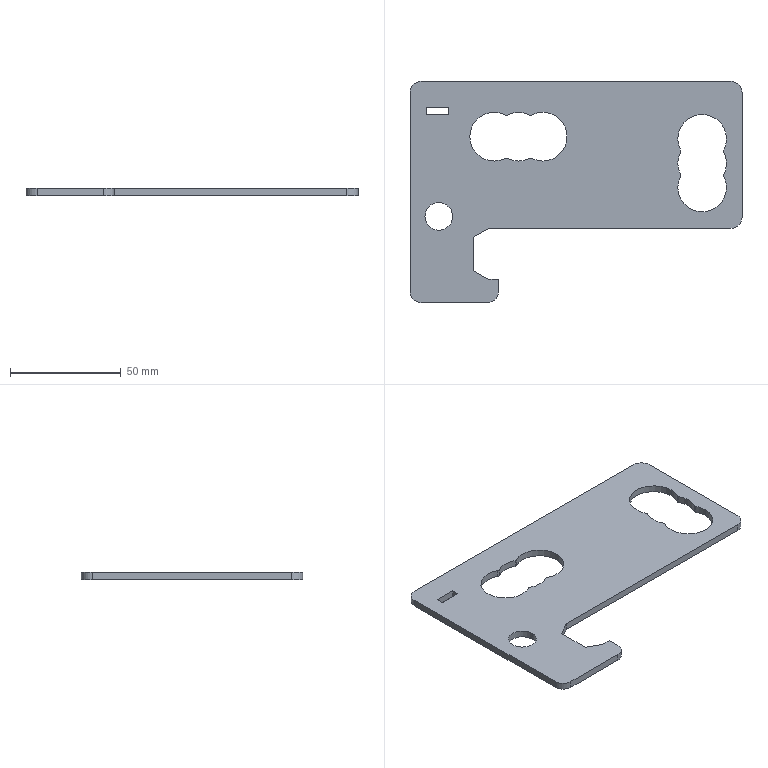Part | SolidWorks | features FlatPattern 1, SMBaseFlange 1, SheetMetal 1 | 1 solid | 47 faces | box 150 x 100 x 3.2 mm | volume 29466 mm3 | cylinder 31 | plane 16 | commonest cylinder face diameters 22 x14 2 x10 10 x5 12.5 x2
STEP:
#1=CARTESIAN_POINT('',(-31.958,111.777,3.2));
#2=VERTEX_POINT('',#1);
#3=CARTESIAN_POINT('',(-48.,102.,3.2));
#4=VERTEX_POINT('',#3);
#5=CARTESIAN_POINT('',(-37.,102.,3.2));
#6=DIRECTION('',(0.,0.,1.));
#7=DIRECTION('',(1.,0.,0.));
#8=AXIS2_PLACEMENT_3D('',#5,#6,#7);
#9=CIRCLE('',#8,11.);
#10=EDGE_CURVE('',#2,#4,#9,.T.);
#11=ORIENTED_EDGE('',*,*,#10,.T.);
#12=CARTESIAN_POINT('',(-48.,102.,0.));
#13=VERTEX_POINT('',#12);
#14=CARTESIAN_POINT('',(-48.,102.,3.2));
#15=DIRECTION('',(0.,0.,-1.));
#16=VECTOR('',#15,1000.);
#17=LINE('',#14,#16);
#18=EDGE_CURVE('',#4,#13,#17,.T.);
#19=ORIENTED_EDGE('',*,*,#18,.T.);
#20=CARTESIAN_POINT('',(-31.958,111.777,0.));
#21=VERTEX_POINT('',#20);
#22=CARTESIAN_POINT('',(-37.,102.,0.));
#23=DIRECTION('',(0.,0.,1.));
#24=DIRECTION('',(1.,0.,0.));
#25=AXIS2_PLACEMENT_3D('',#22,#23,#24);
#26=CIRCLE('',#25,11.);
#27=EDGE_CURVE('',#21,#13,#26,.T.);
#28=ORIENTED_EDGE('',*,*,#27,.F.);
#29=CARTESIAN_POINT('',(-31.958,111.777,3.2));
#30=DIRECTION('',(0.,0.,-1.));
#31=VECTOR('',#30,1000.);
#32=LINE('',#29,#31);
#33=EDGE_CURVE('',#2,#21,#32,.T.);
#34=ORIENTED_EDGE('',*,*,#33,.F.);
#35=EDGE_LOOP('',(#11,#19,#28,#34));
#36=FACE_OUTER_BOUND('',#35,.T.);
#37=CARTESIAN_POINT('',(-37.,102.,3.2));
#38=DIRECTION('',(0.,0.,-1.));
#39=DIRECTION('',(-1.,0.,0.));
#40=AXIS2_PLACEMENT_3D('',#37,#38,#39);
#41=CYLINDRICAL_SURFACE('',#40,11.);
#42=ADVANCED_FACE('',(#36),#41,.F.);
#43=CARTESIAN_POINT('',(46.,79.,3.2));
#44=VERTEX_POINT('',#43);
#45=CARTESIAN_POINT('',(68.,79.,3.2));
#46=VERTEX_POINT('',#45);
#47=CARTESIAN_POINT('',(57.,79.,3.2));
#48=DIRECTION('',(0.,0.,1.));
#49=DIRECTION('',(1.,0.,0.));
#50=AXIS2_PLACEMENT_3D('',#47,#48,#49);
#51=CIRCLE('',#50,11.);
#52=EDGE_CURVE('',#44,#46,#51,.T.);
#53=ORIENTED_EDGE('',*,*,#52,.T.);
#54=CARTESIAN_POINT('',(68.,79.,0.));
#55=VERTEX_POINT('',#54);
#56=CARTESIAN_POINT('',(68.,79.,3.2));
#57=DIRECTION('',(0.,0.,-1.));
#58=VECTOR('',#57,1000.);
#59=LINE('',#56,#58);
#60=EDGE_CURVE('',#46,#55,#59,.T.);
#61=ORIENTED_EDGE('',*,*,#60,.T.);
#62=CARTESIAN_POINT('',(46.,79.,0.));
#63=VERTEX_POINT('',#62);
#64=CARTESIAN_POINT('',(57.,79.,0.));
#65=DIRECTION('',(0.,0.,1.));
#66=DIRECTION('',(1.,0.,0.));
#67=AXIS2_PLACEMENT_3D('',#64,#65,#66);
#68=CIRCLE('',#67,11.);
#69=EDGE_CURVE('',#63,#55,#68,.T.);
#70=ORIENTED_EDGE('',*,*,#69,.F.);
#71=CARTESIAN_POINT('',(46.,79.,3.2));
#72=DIRECTION('',(0.,0.,-1.));
#73=VECTOR('',#72,1000.);
#74=LINE('',#71,#73);
#75=EDGE_CURVE('',#44,#63,#74,.T.);
#76=ORIENTED_EDGE('',*,*,#75,.F.);
#77=EDGE_LOOP('',(#53,#61,#70,#76));
#78=FACE_OUTER_BOUND('',#77,.T.);
#79=CARTESIAN_POINT('',(57.,79.,3.2));
#80=DIRECTION('',(0.,0.,-1.));
#81=DIRECTION('',(-1.,0.,0.));
#82=AXIS2_PLACEMENT_3D('',#79,#80,#81);
#83=CYLINDRICAL_SURFACE('',#82,11.);
#84=ADVANCED_FACE('',(#78),#83,.F.);
#85=CARTESIAN_POINT('',(47.223,84.042,3.2));
#86=VERTEX_POINT('',#85);
#87=CARTESIAN_POINT('',(57.,79.,3.2));
#88=DIRECTION('',(0.,0.,1.));
#89=DIRECTION('',(1.,0.,0.));
#90=AXIS2_PLACEMENT_3D('',#87,#88,#89);
#91=CIRCLE('',#90,11.);
#92=EDGE_CURVE('',#86,#44,#91,.T.);
#93=ORIENTED_EDGE('',*,*,#92,.T.);
#94=ORIENTED_EDGE('',*,*,#75,.T.);
#95=CARTESIAN_POINT('',(47.223,84.042,0.));
#96=VERTEX_POINT('',#95);
#97=CARTESIAN_POINT('',(57.,79.,0.));
#98=DIRECTION('',(0.,0.,1.));
#99=DIRECTION('',(1.,0.,0.));
#100=AXIS2_PLACEMENT_3D('',#97,#98,#99);
#101=CIRCLE('',#100,11.);
#102=EDGE_CURVE('',#96,#63,#101,.T.);
#103=ORIENTED_EDGE('',*,*,#102,.F.);
#104=CARTESIAN_POINT('',(47.223,84.042,3.2));
#105=DIRECTION('',(0.,0.,-1.));
#106=VECTOR('',#105,1000.);
#107=LINE('',#104,#106);
#108=EDGE_CURVE('',#86,#96,#107,.T.);
#109=ORIENTED_EDGE('',*,*,#108,.F.);
#110=EDGE_LOOP('',(#93,#94,#103,#109));
#111=FACE_OUTER_BOUND('',#110,.T.);
#112=CARTESIAN_POINT('',(57.,79.,3.2));
#113=DIRECTION('',(0.,0.,-1.));
#114=DIRECTION('',(-1.,0.,0.));
#115=AXIS2_PLACEMENT_3D('',#112,#113,#114);
#116=CYLINDRICAL_SURFACE('',#115,11.);
#117=ADVANCED_FACE('',(#111),#116,.F.);
#118=CARTESIAN_POINT('',(47.223,95.042,3.2));
#119=VERTEX_POINT('',#118);
#120=CARTESIAN_POINT('',(46.,90.,3.2));
#121=VERTEX_POINT('',#120);
#122=CARTESIAN_POINT('',(57.,90.,3.2));
#123=DIRECTION('',(0.,0.,1.));
#124=DIRECTION('',(1.,0.,0.));
#125=AXIS2_PLACEMENT_3D('',#122,#123,#124);
#126=CIRCLE('',#125,11.);
#127=EDGE_CURVE('',#119,#121,#126,.T.);
#128=ORIENTED_EDGE('',*,*,#127,.T.);
#129=CARTESIAN_POINT('',(46.,90.,0.));
#130=VERTEX_POINT('',#129);
#131=CARTESIAN_POINT('',(46.,90.,3.2));
#132=DIRECTION('',(0.,0.,-1.));
#133=VECTOR('',#132,1000.);
#134=LINE('',#131,#133);
#135=EDGE_CURVE('',#121,#130,#134,.T.);
#136=ORIENTED_EDGE('',*,*,#135,.T.);
#137=CARTESIAN_POINT('',(47.223,95.042,0.));
#138=VERTEX_POINT('',#137);
#139=CARTESIAN_POINT('',(57.,90.,0.));
#140=DIRECTION('',(0.,0.,1.));
#141=DIRECTION('',(1.,0.,0.));
#142=AXIS2_PLACEMENT_3D('',#139,#140,#141);
#143=CIRCLE('',#142,11.);
#144=EDGE_CURVE('',#138,#130,#143,.T.);
#145=ORIENTED_EDGE('',*,*,#144,.F.);
#146=CARTESIAN_POINT('',(47.223,95.042,3.2));
#147=DIRECTION('',(0.,0.,-1.));
#148=VECTOR('',#147,1000.);
#149=LINE('',#146,#148);
#150=EDGE_CURVE('',#119,#138,#149,.T.);
#151=ORIENTED_EDGE('',*,*,#150,.F.);
#152=EDGE_LOOP('',(#128,#136,#145,#151));
#153=FACE_OUTER_BOUND('',#152,.T.);
#154=CARTESIAN_POINT('',(57.,90.,3.2));
#155=DIRECTION('',(0.,0.,-1.));
#156=DIRECTION('',(-1.,0.,0.));
#157=AXIS2_PLACEMENT_3D('',#154,#155,#156);
#158=CYLINDRICAL_SURFACE('',#157,11.);
#159=ADVANCED_FACE('',(#153),#158,.F.);
#160=CARTESIAN_POINT('',(66.777,95.958,3.2));
#161=VERTEX_POINT('',#160);
#162=CARTESIAN_POINT('',(68.,101.,3.2));
#163=VERTEX_POINT('',#162);
#164=CARTESIAN_POINT('',(57.,101.,3.2));
#165=DIRECTION('',(0.,0.,1.));
#166=DIRECTION('',(1.,0.,0.));
#167=AXIS2_PLACEMENT_3D('',#164,#165,#166);
#168=CIRCLE('',#167,11.);
#169=EDGE_CURVE('',#161,#163,#168,.T.);
#170=ORIENTED_EDGE('',*,*,#169,.T.);
#171=CARTESIAN_POINT('',(68.,101.,0.));
#172=VERTEX_POINT('',#171);
#173=CARTESIAN_POINT('',(68.,101.,3.2));
#174=DIRECTION('',(0.,0.,-1.));
#175=VECTOR('',#174,1000.);
#176=LINE('',#173,#175);
#177=EDGE_CURVE('',#163,#172,#176,.T.);
#178=ORIENTED_EDGE('',*,*,#177,.T.);
#179=CARTESIAN_POINT('',(66.777,95.958,0.));
#180=VERTEX_POINT('',#179);
#181=CARTESIAN_POINT('',(57.,101.,0.));
#182=DIRECTION('',(0.,0.,1.));
#183=DIRECTION('',(1.,0.,0.));
#184=AXIS2_PLACEMENT_3D('',#181,#182,#183);
#185=CIRCLE('',#184,11.);
#186=EDGE_CURVE('',#180,#172,#185,.T.);
#187=ORIENTED_EDGE('',*,*,#186,.F.);
#188=CARTESIAN_POINT('',(66.777,95.958,3.2));
#189=DIRECTION('',(0.,0.,-1.));
#190=VECTOR('',#189,1000.);
#191=LINE('',#188,#190);
#192=EDGE_CURVE('',#161,#180,#191,.T.);
#193=ORIENTED_EDGE('',*,*,#192,.F.);
#194=EDGE_LOOP('',(#170,#178,#187,#193));
#195=FACE_OUTER_BOUND('',#194,.T.);
#196=CARTESIAN_POINT('',(57.,101.,3.2));
#197=DIRECTION('',(0.,0.,-1.));
#198=DIRECTION('',(-1.,0.,0.));
#199=AXIS2_PLACEMENT_3D('',#196,#197,#198);
#200=CYLINDRICAL_SURFACE('',#199,11.);
#201=ADVANCED_FACE('',(#195),#200,.F.);
#202=ORIENTED_EDGE('',*,*,#177,.F.);
#203=CARTESIAN_POINT('',(46.,101.,3.2));
#204=VERTEX_POINT('',#203);
#205=CARTESIAN_POINT('',(57.,101.,3.2));
#206=DIRECTION('',(0.,0.,1.));
#207=DIRECTION('',(1.,0.,0.));
#208=AXIS2_PLACEMENT_3D('',#205,#206,#207);
#209=CIRCLE('',#208,11.);
#210=EDGE_CURVE('',#163,#204,#209,.T.);
#211=ORIENTED_EDGE('',*,*,#210,.T.);
#212=CARTESIAN_POINT('',(46.,101.,0.));
#213=VERTEX_POINT('',#212);
#214=CARTESIAN_POINT('',(46.,101.,3.2));
#215=DIRECTION('',(0.,0.,-1.));
#216=VECTOR('',#215,1000.);
#217=LINE('',#214,#216);
#218=EDGE_CURVE('',#204,#213,#217,.T.);
#219=ORIENTED_EDGE('',*,*,#218,.T.);
#220=CARTESIAN_POINT('',(57.,101.,0.));
#221=DIRECTION('',(0.,0.,1.));
#222=DIRECTION('',(1.,0.,0.));
#223=AXIS2_PLACEMENT_3D('',#220,#221,#222);
#224=CIRCLE('',#223,11.);
#225=EDGE_CURVE('',#172,#213,#224,.T.);
#226=ORIENTED_EDGE('',*,*,#225,.F.);
#227=EDGE_LOOP('',(#202,#211,#219,#226));
#228=FACE_OUTER_BOUND('',#227,.T.);
#229=CARTESIAN_POINT('',(57.,101.,3.2));
#230=DIRECTION('',(0.,0.,-1.));
#231=DIRECTION('',(-1.,0.,0.));
#232=AXIS2_PLACEMENT_3D('',#229,#230,#231);
#233=CYLINDRICAL_SURFACE('',#232,11.);
#234=ADVANCED_FACE('',(#228),#233,.F.);
#235=CARTESIAN_POINT('',(66.777,95.042,3.2));
#236=VERTEX_POINT('',#235);
#237=CARTESIAN_POINT('',(66.665,95.5,3.2));
#238=VERTEX_POINT('',#237);
#239=CARTESIAN_POINT('',(67.665,95.5,3.2));
#240=DIRECTION('',(0.,0.,-1.));
#241=DIRECTION('',(1.,0.,0.));
#242=AXIS2_PLACEMENT_3D('',#239,#240,#241);
#243=CIRCLE('',#242,1.);
#244=EDGE_CURVE('',#236,#238,#243,.T.);
#245=ORIENTED_EDGE('',*,*,#244,.T.);
#246=CARTESIAN_POINT('',(66.665,95.5,0.));
#247=VERTEX_POINT('',#246);
#248=CARTESIAN_POINT('',(66.665,95.5,3.2));
#249=DIRECTION('',(0.,0.,-1.));
#250=VECTOR('',#249,1000.);
#251=LINE('',#248,#250);
#252=EDGE_CURVE('',#238,#247,#251,.T.);
#253=ORIENTED_EDGE('',*,*,#252,.T.);
#254=CARTESIAN_POINT('',(66.777,95.042,0.));
#255=VERTEX_POINT('',#254);
#256=CARTESIAN_POINT('',(67.665,95.5,0.));
#257=DIRECTION('',(0.,0.,-1.));
#258=DIRECTION('',(1.,0.,0.));
#259=AXIS2_PLACEMENT_3D('',#256,#257,#258);
#260=CIRCLE('',#259,1.);
#261=EDGE_CURVE('',#255,#247,#260,.T.);
#262=ORIENTED_EDGE('',*,*,#261,.F.);
#263=CARTESIAN_POINT('',(66.777,95.042,3.2));
#264=DIRECTION('',(0.,0.,-1.));
#265=VECTOR('',#264,1000.);
#266=LINE('',#263,#265);
#267=EDGE_CURVE('',#236,#255,#266,.T.);
#268=ORIENTED_EDGE('',*,*,#267,.F.);
#269=EDGE_LOOP('',(#245,#253,#262,#268));
#270=FACE_OUTER_BOUND('',#269,.T.);
#271=CARTESIAN_POINT('',(67.665,95.5,3.2));
#272=DIRECTION('',(0.,0.,-1.));
#273=DIRECTION('',(-1.,0.,0.));
#274=AXIS2_PLACEMENT_3D('',#271,#272,#273);
#275=CYLINDRICAL_SURFACE('',#274,1.);
#276=ADVANCED_FACE('',(#270),#275,.T.);
#277=CARTESIAN_POINT('',(66.777,84.042,3.2));
#278=VERTEX_POINT('',#277);
#279=CARTESIAN_POINT('',(66.665,84.5,3.2));
#280=VERTEX_POINT('',#279);
#281=CARTESIAN_POINT('',(67.665,84.5,3.2));
#282=DIRECTION('',(0.,0.,-1.));
#283=DIRECTION('',(-1.,0.,0.));
#284=AXIS2_PLACEMENT_3D('',#281,#282,#283);
#285=CIRCLE('',#284,1.);
#286=EDGE_CURVE('',#278,#280,#285,.T.);
#287=ORIENTED_EDGE('',*,*,#286,.T.);
#288=CARTESIAN_POINT('',(66.665,84.5,0.));
#289=VERTEX_POINT('',#288);
#290=CARTESIAN_POINT('',(66.665,84.5,3.2));
#291=DIRECTION('',(0.,0.,-1.));
#292=VECTOR('',#291,1000.);
#293=LINE('',#290,#292);
#294=EDGE_CURVE('',#280,#289,#293,.T.);
#295=ORIENTED_EDGE('',*,*,#294,.T.);
#296=CARTESIAN_POINT('',(66.777,84.042,0.));
#297=VERTEX_POINT('',#296);
#298=CARTESIAN_POINT('',(67.665,84.5,0.));
#299=DIRECTION('',(0.,0.,-1.));
#300=DIRECTION('',(-1.,0.,0.));
#301=AXIS2_PLACEMENT_3D('',#298,#299,#300);
#302=CIRCLE('',#301,1.);
#303=EDGE_CURVE('',#297,#289,#302,.T.);
#304=ORIENTED_EDGE('',*,*,#303,.F.);
#305=CARTESIAN_POINT('',(66.777,84.042,3.2));
#306=DIRECTION('',(0.,0.,-1.));
#307=VECTOR('',#306,1000.);
#308=LINE('',#305,#307);
#309=EDGE_CURVE('',#278,#297,#308,.T.);
#310=ORIENTED_EDGE('',*,*,#309,.F.);
#311=EDGE_LOOP('',(#287,#295,#304,#310));
#312=FACE_OUTER_BOUND('',#311,.T.);
#313=CARTESIAN_POINT('',(67.665,84.5,3.2));
#314=DIRECTION('',(0.,0.,-1.));
#315=DIRECTION('',(-1.,0.,0.));
#316=AXIS2_PLACEMENT_3D('',#313,#314,#315);
#317=CYLINDRICAL_SURFACE('',#316,1.);
#318=ADVANCED_FACE('',(#312),#317,.T.);
#319=CARTESIAN_POINT('',(-68.25,66.,3.2));
#320=VERTEX_POINT('',#319);
#321=CARTESIAN_POINT('',(-55.75,66.,3.2));
#322=VERTEX_POINT('',#321);
#323=CARTESIAN_POINT('',(-62.,66.,3.2));
#324=DIRECTION('',(0.,0.,1.));
#325=DIRECTION('',(1.,0.,0.));
#326=AXIS2_PLACEMENT_3D('',#323,#324,#325);
#327=CIRCLE('',#326,6.25);
#328=EDGE_CURVE('',#320,#322,#327,.T.);
#329=ORIENTED_EDGE('',*,*,#328,.T.);
#330=CARTESIAN_POINT('',(-55.75,66.,0.));
#331=VERTEX_POINT('',#330);
#332=CARTESIAN_POINT('',(-55.75,66.,3.2));
#333=DIRECTION('',(0.,0.,-1.));
#334=VECTOR('',#333,1000.);
#335=LINE('',#332,#334);
#336=EDGE_CURVE('',#322,#331,#335,.T.);
#337=ORIENTED_EDGE('',*,*,#336,.T.);
#338=CARTESIAN_POINT('',(-68.25,66.,0.));
#339=VERTEX_POINT('',#338);
#340=CARTESIAN_POINT('',(-62.,66.,0.));
#341=DIRECTION('',(0.,0.,1.));
#342=DIRECTION('',(1.,0.,0.));
#343=AXIS2_PLACEMENT_3D('',#340,#341,#342);
#344=CIRCLE('',#343,6.25);
#345=EDGE_CURVE('',#339,#331,#344,.T.);
#346=ORIENTED_EDGE('',*,*,#345,.F.);
#347=CARTESIAN_POINT('',(-68.25,66.,3.2));
#348=DIRECTION('',(0.,0.,-1.));
#349=VECTOR('',#348,1000.);
#350=LINE('',#347,#349);
#351=EDGE_CURVE('',#320,#339,#350,.T.);
#352=ORIENTED_EDGE('',*,*,#351,.F.);
#353=EDGE_LOOP('',(#329,#337,#346,#352));
#354=FACE_OUTER_BOUND('',#353,.T.);
#355=CARTESIAN_POINT('',(-62.,66.,3.2));
#356=DIRECTION('',(0.,0.,-1.));
#357=DIRECTION('',(-1.,0.,0.));
#358=AXIS2_PLACEMENT_3D('',#355,#356,#357);
#359=CYLINDRICAL_SURFACE('',#358,6.25);
#360=ADVANCED_FACE('',(#354),#359,.F.);
#361=CARTESIAN_POINT('',(-20.958,92.223,3.2));
#362=VERTEX_POINT('',#361);
#363=CARTESIAN_POINT('',(-20.042,92.223,3.2));
#364=VERTEX_POINT('',#363);
#365=CARTESIAN_POINT('',(-20.5,91.335,3.2));
#366=DIRECTION('',(0.,0.,-1.));
#367=DIRECTION('',(1.,0.,0.));
#368=AXIS2_PLACEMENT_3D('',#365,#366,#367);
#369=CIRCLE('',#368,1.);
#370=EDGE_CURVE('',#362,#364,#369,.T.);
#371=ORIENTED_EDGE('',*,*,#370,.F.);
#372=CARTESIAN_POINT('',(-31.042,92.223,3.2));
#373=VERTEX_POINT('',#372);
#374=CARTESIAN_POINT('',(-26.,102.,3.2));
#375=DIRECTION('',(0.,0.,1.));
#376=DIRECTION('',(1.,0.,0.));
#377=AXIS2_PLACEMENT_3D('',#374,#375,#376);
#378=CIRCLE('',#377,11.);
#379=EDGE_CURVE('',#373,#362,#378,.T.);
#380=ORIENTED_EDGE('',*,*,#379,.F.);
#381=CARTESIAN_POINT('',(-31.958,92.223,3.2));
#382=VERTEX_POINT('',#381);
#383=CARTESIAN_POINT('',(-31.5,91.335,3.2));
#384=DIRECTION('',(0.,0.,-1.));
#385=DIRECTION('',(-1.,0.,0.));
#386=AXIS2_PLACEMENT_3D('',#383,#384,#385);
#387=CIRCLE('',#386,1.);
#388=EDGE_CURVE('',#382,#373,#387,.T.);
#389=ORIENTED_EDGE('',*,*,#388,.F.);
#390=CARTESIAN_POINT('',(-37.,102.,3.2));
#391=DIRECTION('',(0.,0.,1.));
#392=DIRECTION('',(1.,0.,0.));
#393=AXIS2_PLACEMENT_3D('',#390,#391,#392);
#394=CIRCLE('',#393,11.);
#395=EDGE_CURVE('',#4,#382,#394,.T.);
#396=ORIENTED_EDGE('',*,*,#395,.F.);
#397=ORIENTED_EDGE('',*,*,#10,.F.);
#398=CARTESIAN_POINT('',(-31.042,111.777,3.2));
#399=VERTEX_POINT('',#398);
#400=CARTESIAN_POINT('',(-31.5,112.665,3.2));
#401=DIRECTION('',(0.,0.,-1.));
#402=DIRECTION('',(1.,0.,0.));
#403=AXIS2_PLACEMENT_3D('',#400,#401,#402);
#404=CIRCLE('',#403,1.);
#405=EDGE_CURVE('',#399,#2,#404,.T.);
#406=ORIENTED_EDGE('',*,*,#405,.F.);
#407=CARTESIAN_POINT('',(-20.958,111.777,3.2));
#408=VERTEX_POINT('',#407);
#409=CARTESIAN_POINT('',(-26.,102.,3.2));
#410=DIRECTION('',(0.,0.,1.));
#411=DIRECTION('',(1.,0.,0.));
#412=AXIS2_PLACEMENT_3D('',#409,#410,#411);
#413=CIRCLE('',#412,11.);
#414=EDGE_CURVE('',#408,#399,#413,.T.);
#415=ORIENTED_EDGE('',*,*,#414,.F.);
#416=CARTESIAN_POINT('',(-20.042,111.777,3.2));
#417=VERTEX_POINT('',#416);
#418=CARTESIAN_POINT('',(-20.5,112.665,3.2));
#419=DIRECTION('',(0.,0.,-1.));
#420=DIRECTION('',(-1.,0.,0.));
#421=AXIS2_PLACEMENT_3D('',#418,#419,#420);
#422=CIRCLE('',#421,1.);
#423=EDGE_CURVE('',#417,#408,#422,.T.);
#424=ORIENTED_EDGE('',*,*,#423,.F.);
#425=CARTESIAN_POINT('',(-15.,102.,3.2));
#426=DIRECTION('',(0.,0.,1.));
#427=DIRECTION('',(1.,0.,0.));
#428=AXIS2_PLACEMENT_3D('',#425,#426,#427);
#429=CIRCLE('',#428,11.);
#430=EDGE_CURVE('',#364,#417,#429,.T.);
#431=ORIENTED_EDGE('',*,*,#430,.F.);
#432=EDGE_LOOP('',(#371,#380,#389,#396,#397,#406,#415,#424,#431));
#433=FACE_BOUND('',#432,.T.);
#434=ORIENTED_EDGE('',*,*,#328,.F.);
#435=CARTESIAN_POINT('',(-62.,66.,3.2));
#436=DIRECTION('',(0.,0.,1.));
#437=DIRECTION('',(1.,0.,0.));
#438=AXIS2_PLACEMENT_3D('',#435,#436,#437);
#439=CIRCLE('',#438,6.25);
#440=EDGE_CURVE('',#322,#320,#439,.T.);
#441=ORIENTED_EDGE('',*,*,#440,.F.);
#442=EDGE_LOOP('',(#434,#441));
#443=FACE_BOUND('',#442,.T.);
#444=CARTESIAN_POINT('',(-46.4,56.62,3.2));
#445=VERTEX_POINT('',#444);
#446=CARTESIAN_POINT('',(-39.41,60.53,3.2));
#447=VERTEX_POINT('',#446);
#448=CARTESIAN_POINT('',(-39.41,60.53,3.2));
#449=DIRECTION('',(0.8727,0.4882,0.));
#450=VECTOR('',#449,1000.);
#451=LINE('',#448,#450);
#452=EDGE_CURVE('',#445,#447,#451,.T.);
#453=ORIENTED_EDGE('',*,*,#452,.T.);
#454=CARTESIAN_POINT('',(70.,60.53,3.2));
#455=VERTEX_POINT('',#454);
#456=CARTESIAN_POINT('',(-39.41,60.53,3.2));
#457=DIRECTION('',(1.,0.,0.));
#458=VECTOR('',#457,1000.);
#459=LINE('',#456,#458);
#460=EDGE_CURVE('',#447,#455,#459,.T.);
#461=ORIENTED_EDGE('',*,*,#460,.T.);
#462=CARTESIAN_POINT('',(75.,65.53,3.2));
#463=VERTEX_POINT('',#462);
#464=CARTESIAN_POINT('',(70.,65.53,3.2));
#465=DIRECTION('',(0.,0.,1.));
#466=DIRECTION('',(-1.,0.,0.));
#467=AXIS2_PLACEMENT_3D('',#464,#465,#466);
#468=CIRCLE('',#467,5.);
#469=EDGE_CURVE('',#455,#463,#468,.T.);
#470=ORIENTED_EDGE('',*,*,#469,.T.);
#471=CARTESIAN_POINT('',(75.,122.,3.2));
#472=VERTEX_POINT('',#471);
#473=CARTESIAN_POINT('',(75.,122.,3.2));
#474=DIRECTION('',(0.,1.,0.));
#475=VECTOR('',#474,1000.);
#476=LINE('',#473,#475);
#477=EDGE_CURVE('',#463,#472,#476,.T.);
#478=ORIENTED_EDGE('',*,*,#477,.T.);
#479=CARTESIAN_POINT('',(70.,127.,3.2));
#480=VERTEX_POINT('',#479);
#481=CARTESIAN_POINT('',(70.,122.,3.2));
#482=DIRECTION('',(0.,0.,1.));
#483=DIRECTION('',(1.,0.,0.));
#484=AXIS2_PLACEMENT_3D('',#481,#482,#483);
#485=CIRCLE('',#484,5.);
#486=EDGE_CURVE('',#472,#480,#485,.T.);
#487=ORIENTED_EDGE('',*,*,#486,.T.);
#488=CARTESIAN_POINT('',(-70.,127.,3.2));
#489=VERTEX_POINT('',#488);
#490=CARTESIAN_POINT('',(-70.,127.,3.2));
#491=DIRECTION('',(-1.,0.,0.));
#492=VECTOR('',#491,1000.);
#493=LINE('',#490,#492);
#494=EDGE_CURVE('',#480,#489,#493,.T.);
#495=ORIENTED_EDGE('',*,*,#494,.T.);
#496=CARTESIAN_POINT('',(-75.,122.,3.2));
#497=VERTEX_POINT('',#496);
#498=CARTESIAN_POINT('',(-70.,122.,3.2));
#499=DIRECTION('',(0.,0.,1.));
#500=DIRECTION('',(-1.,0.,0.));
#501=AXIS2_PLACEMENT_3D('',#498,#499,#500);
#502=CIRCLE('',#501,5.);
#503=EDGE_CURVE('',#489,#497,#502,.T.);
#504=ORIENTED_EDGE('',*,*,#503,.T.);
#505=CARTESIAN_POINT('',(-75.,32.,3.2));
#506=VERTEX_POINT('',#505);
#507=CARTESIAN_POINT('',(-75.,32.,3.2));
#508=DIRECTION('',(0.,-1.,0.));
#509=VECTOR('',#508,1000.);
#510=LINE('',#507,#509);
#511=EDGE_CURVE('',#497,#506,#510,.T.);
#512=ORIENTED_EDGE('',*,*,#511,.T.);
#513=CARTESIAN_POINT('',(-70.,27.,3.2));
#514=VERTEX_POINT('',#513);
#515=CARTESIAN_POINT('',(-70.,32.,3.2));
#516=DIRECTION('',(0.,0.,1.));
#517=DIRECTION('',(-1.,0.,0.));
#518=AXIS2_PLACEMENT_3D('',#515,#516,#517);
#519=CIRCLE('',#518,5.);
#520=EDGE_CURVE('',#506,#514,#519,.T.);
#521=ORIENTED_EDGE('',*,*,#520,.T.);
#522=CARTESIAN_POINT('',(-40.,27.,3.2));
#523=VERTEX_POINT('',#522);
#524=CARTESIAN_POINT('',(-40.,27.,3.2));
#525=DIRECTION('',(1.,0.,0.));
#526=VECTOR('',#525,1000.);
#527=LINE('',#524,#526);
#528=EDGE_CURVE('',#514,#523,#527,.T.);
#529=ORIENTED_EDGE('',*,*,#528,.T.);
#530=CARTESIAN_POINT('',(-35.,32.,3.2));
#531=VERTEX_POINT('',#530);
#532=CARTESIAN_POINT('',(-40.,32.,3.2));
#533=DIRECTION('',(0.,0.,1.));
#534=DIRECTION('',(-1.,0.,0.));
#535=AXIS2_PLACEMENT_3D('',#532,#533,#534);
#536=CIRCLE('',#535,5.);
#537=EDGE_CURVE('',#523,#531,#536,.T.);
#538=ORIENTED_EDGE('',*,*,#537,.T.);
#539=CARTESIAN_POINT('',(-35.,37.47,3.2));
#540=VERTEX_POINT('',#539);
#541=CARTESIAN_POINT('',(-35.,37.47,3.2));
#542=DIRECTION('',(0.,1.,0.));
#543=VECTOR('',#542,1000.);
#544=LINE('',#541,#543);
#545=EDGE_CURVE('',#531,#540,#544,.T.);
#546=ORIENTED_EDGE('',*,*,#545,.T.);
#547=CARTESIAN_POINT('',(-39.41,37.47,3.2));
#548=VERTEX_POINT('',#547);
#549=CARTESIAN_POINT('',(-39.41,37.47,3.2));
#550=DIRECTION('',(-1.,0.,0.));
#551=VECTOR('',#550,1000.);
#552=LINE('',#549,#551);
#553=EDGE_CURVE('',#540,#548,#552,.T.);
#554=ORIENTED_EDGE('',*,*,#553,.T.);
#555=CARTESIAN_POINT('',(-46.4,41.38,3.2));
#556=VERTEX_POINT('',#555);
#557=CARTESIAN_POINT('',(-46.4,41.38,3.2));
#558=DIRECTION('',(-0.8727,0.4882,0.));
#559=VECTOR('',#558,1000.);
#560=LINE('',#557,#559);
#561=EDGE_CURVE('',#548,#556,#560,.T.);
#562=ORIENTED_EDGE('',*,*,#561,.T.);
#563=CARTESIAN_POINT('',(-46.4,56.62,3.2));
#564=DIRECTION('',(0.,1.,0.));
#565=VECTOR('',#564,1000.);
#566=LINE('',#563,#565);
#567=EDGE_CURVE('',#556,#445,#566,.T.);
#568=ORIENTED_EDGE('',*,*,#567,.T.);
#569=EDGE_LOOP('',(#453,#461,#470,#478,#487,#495,#504,#512,#521,#529,#538,#546,#554,#562,#568));
#570=FACE_OUTER_BOUND('',#569,.T.);
#571=ORIENTED_EDGE('',*,*,#286,.F.);
#572=CARTESIAN_POINT('',(57.,79.,3.2));
#573=DIRECTION('',(0.,0.,1.));
#574=DIRECTION('',(1.,0.,0.));
#575=AXIS2_PLACEMENT_3D('',#572,#573,#574);
#576=CIRCLE('',#575,11.);
#577=EDGE_CURVE('',#46,#278,#576,.T.);
#578=ORIENTED_EDGE('',*,*,#577,.F.);
#579=ORIENTED_EDGE('',*,*,#52,.F.);
#580=ORIENTED_EDGE('',*,*,#92,.F.);
#581=CARTESIAN_POINT('',(47.223,84.958,3.2));
#582=VERTEX_POINT('',#581);
#583=CARTESIAN_POINT('',(46.335,84.5,3.2));
#584=DIRECTION('',(0.,0.,-1.));
#585=DIRECTION('',(1.,0.,0.));
#586=AXIS2_PLACEMENT_3D('',#583,#584,#585);
#587=CIRCLE('',#586,1.);
#588=EDGE_CURVE('',#582,#86,#587,.T.);
#589=ORIENTED_EDGE('',*,*,#588,.F.);
#590=CARTESIAN_POINT('',(57.,90.,3.2));
#591=DIRECTION('',(0.,0.,1.));
#592=DIRECTION('',(1.,0.,0.));
#593=AXIS2_PLACEMENT_3D('',#590,#591,#592);
#594=CIRCLE('',#593,11.);
#595=EDGE_CURVE('',#121,#582,#594,.T.);
#596=ORIENTED_EDGE('',*,*,#595,.F.);
#597=ORIENTED_EDGE('',*,*,#127,.F.);
#598=CARTESIAN_POINT('',(47.223,95.958,3.2));
#599=VERTEX_POINT('',#598);
#600=CARTESIAN_POINT('',(46.335,95.5,3.2));
#601=DIRECTION('',(0.,0.,-1.));
#602=DIRECTION('',(-1.,0.,0.));
#603=AXIS2_PLACEMENT_3D('',#600,#601,#602);
#604=CIRCLE('',#603,1.);
#605=EDGE_CURVE('',#599,#119,#604,.T.);
#606=ORIENTED_EDGE('',*,*,#605,.F.);
#607=CARTESIAN_POINT('',(57.,101.,3.2));
#608=DIRECTION('',(0.,0.,1.));
#609=DIRECTION('',(1.,0.,0.));
#610=AXIS2_PLACEMENT_3D('',#607,#608,#609);
#611=CIRCLE('',#610,11.);
#612=EDGE_CURVE('',#204,#599,#611,.T.);
#613=ORIENTED_EDGE('',*,*,#612,.F.);
#614=ORIENTED_EDGE('',*,*,#210,.F.);
#615=ORIENTED_EDGE('',*,*,#169,.F.);
#616=CARTESIAN_POINT('',(67.665,95.5,3.2));
#617=DIRECTION('',(0.,0.,-1.));
#618=DIRECTION('',(1.,0.,0.));
#619=AXIS2_PLACEMENT_3D('',#616,#617,#618);
#620=CIRCLE('',#619,1.);
#621=EDGE_CURVE('',#238,#161,#620,.T.);
#622=ORIENTED_EDGE('',*,*,#621,.F.);
#623=ORIENTED_EDGE('',*,*,#244,.F.);
#624=CARTESIAN_POINT('',(66.777,84.958,3.2));
#625=VERTEX_POINT('',#624);
#626=CARTESIAN_POINT('',(57.,90.,3.2));
#627=DIRECTION('',(0.,0.,1.));
#628=DIRECTION('',(1.,0.,0.));
#629=AXIS2_PLACEMENT_3D('',#626,#627,#628);
#630=CIRCLE('',#629,11.);
#631=EDGE_CURVE('',#625,#236,#630,.T.);
#632=ORIENTED_EDGE('',*,*,#631,.F.);
#633=CARTESIAN_POINT('',(67.665,84.5,3.2));
#634=DIRECTION('',(0.,0.,-1.));
#635=DIRECTION('',(-1.,0.,0.));
#636=AXIS2_PLACEMENT_3D('',#633,#634,#635);
#637=CIRCLE('',#636,1.);
#638=EDGE_CURVE('',#280,#625,#637,.T.);
#639=ORIENTED_EDGE('',*,*,#638,.F.);
#640=EDGE_LOOP('',(#571,#578,#579,#580,#589,#596,#597,#606,#613,#614,#615,#622,#623,#632,#639));
#641=FACE_BOUND('',#640,.T.);
#642=CARTESIAN_POINT('',(-67.5,115.,3.2));
#643=VERTEX_POINT('',#642);
#644=CARTESIAN_POINT('',(-67.5,111.8,3.2));
#645=VERTEX_POINT('',#644);
#646=CARTESIAN_POINT('',(-67.5,115.,3.2));
#647=DIRECTION('',(0.,-1.,0.));
#648=VECTOR('',#647,1000.);
#649=LINE('',#646,#648);
#650=EDGE_CURVE('',#643,#645,#649,.T.);
#651=ORIENTED_EDGE('',*,*,#650,.F.);
#652=CARTESIAN_POINT('',(-57.5,115.,3.2));
#653=VERTEX_POINT('',#652);
#654=CARTESIAN_POINT('',(-67.5,115.,3.2));
#655=DIRECTION('',(-1.,0.,0.));
#656=VECTOR('',#655,1000.);
#657=LINE('',#654,#656);
#658=EDGE_CURVE('',#653,#643,#657,.T.);
#659=ORIENTED_EDGE('',*,*,#658,.F.);
#660=CARTESIAN_POINT('',(-57.5,111.8,3.2));
#661=VERTEX_POINT('',#660);
#662=CARTESIAN_POINT('',(-57.5,115.,3.2));
#663=DIRECTION('',(0.,1.,0.));
#664=VECTOR('',#663,1000.);
#665=LINE('',#662,#664);
#666=EDGE_CURVE('',#661,#653,#665,.T.);
#667=ORIENTED_EDGE('',*,*,#666,.F.);
#668=CARTESIAN_POINT('',(-67.5,111.8,3.2));
#669=DIRECTION('',(1.,0.,0.));
#670=VECTOR('',#669,1000.);
#671=LINE('',#668,#670);
#672=EDGE_CURVE('',#645,#661,#671,.T.);
#673=ORIENTED_EDGE('',*,*,#672,.F.);
#674=EDGE_LOOP('',(#651,#659,#667,#673));
#675=FACE_BOUND('',#674,.T.);
#676=CARTESIAN_POINT('',(-40.,32.,3.2));
#677=DIRECTION('',(0.,0.,-1.));
#678=DIRECTION('',(-1.,0.,0.));
#679=AXIS2_PLACEMENT_3D('',#676,#677,#678);
#680=PLANE('',#679);
#681=ADVANCED_FACE('',(#433,#443,#570,#641,#675),#680,.F.);
#682=CARTESIAN_POINT('',(-46.4,56.62,0.));
#683=VERTEX_POINT('',#682);
#684=CARTESIAN_POINT('',(-39.41,60.53,0.));
#685=VERTEX_POINT('',#684);
#686=CARTESIAN_POINT('',(-39.41,60.53,0.));
#687=DIRECTION('',(0.8727,0.4882,0.));
#688=VECTOR('',#687,1000.);
#689=LINE('',#686,#688);
#690=EDGE_CURVE('',#683,#685,#689,.T.);
#691=ORIENTED_EDGE('',*,*,#690,.F.);
#692=CARTESIAN_POINT('',(-46.4,41.38,0.));
#693=VERTEX_POINT('',#692);
#694=CARTESIAN_POINT('',(-46.4,56.62,0.));
#695=DIRECTION('',(0.,1.,0.));
#696=VECTOR('',#695,1000.);
#697=LINE('',#694,#696);
#698=EDGE_CURVE('',#693,#683,#697,.T.);
#699=ORIENTED_EDGE('',*,*,#698,.F.);
#700=CARTESIAN_POINT('',(-39.41,37.47,0.));
#701=VERTEX_POINT('',#700);
#702=CARTESIAN_POINT('',(-46.4,41.38,0.));
#703=DIRECTION('',(-0.8727,0.4882,0.));
#704=VECTOR('',#703,1000.);
#705=LINE('',#702,#704);
#706=EDGE_CURVE('',#701,#693,#705,.T.);
#707=ORIENTED_EDGE('',*,*,#706,.F.);
#708=CARTESIAN_POINT('',(-35.,37.47,0.));
#709=VERTEX_POINT('',#708);
#710=CARTESIAN_POINT('',(-39.41,37.47,0.));
#711=DIRECTION('',(-1.,0.,0.));
#712=VECTOR('',#711,1000.);
#713=LINE('',#710,#712);
#714=EDGE_CURVE('',#709,#701,#713,.T.);
#715=ORIENTED_EDGE('',*,*,#714,.F.);
#716=CARTESIAN_POINT('',(-35.,32.,0.));
#717=VERTEX_POINT('',#716);
#718=CARTESIAN_POINT('',(-35.,37.47,0.));
#719=DIRECTION('',(0.,1.,0.));
#720=VECTOR('',#719,1000.);
#721=LINE('',#718,#720);
#722=EDGE_CURVE('',#717,#709,#721,.T.);
#723=ORIENTED_EDGE('',*,*,#722,.F.);
#724=CARTESIAN_POINT('',(-40.,27.,0.));
#725=VERTEX_POINT('',#724);
#726=CARTESIAN_POINT('',(-40.,32.,0.));
#727=DIRECTION('',(0.,0.,1.));
#728=DIRECTION('',(-1.,0.,0.));
#729=AXIS2_PLACEMENT_3D('',#726,#727,#728);
#730=CIRCLE('',#729,5.);
#731=EDGE_CURVE('',#725,#717,#730,.T.);
#732=ORIENTED_EDGE('',*,*,#731,.F.);
#733=CARTESIAN_POINT('',(-70.,27.,0.));
#734=VERTEX_POINT('',#733);
#735=CARTESIAN_POINT('',(-40.,27.,0.));
#736=DIRECTION('',(1.,0.,0.));
#737=VECTOR('',#736,1000.);
#738=LINE('',#735,#737);
#739=EDGE_CURVE('',#734,#725,#738,.T.);
#740=ORIENTED_EDGE('',*,*,#739,.F.);
#741=CARTESIAN_POINT('',(-75.,32.,0.));
#742=VERTEX_POINT('',#741);
#743=CARTESIAN_POINT('',(-70.,32.,0.));
#744=DIRECTION('',(0.,0.,1.));
#745=DIRECTION('',(-1.,0.,0.));
#746=AXIS2_PLACEMENT_3D('',#743,#744,#745);
#747=CIRCLE('',#746,5.);
#748=EDGE_CURVE('',#742,#734,#747,.T.);
#749=ORIENTED_EDGE('',*,*,#748,.F.);
#750=CARTESIAN_POINT('',(-75.,122.,0.));
#751=VERTEX_POINT('',#750);
#752=CARTESIAN_POINT('',(-75.,32.,0.));
#753=DIRECTION('',(0.,-1.,0.));
#754=VECTOR('',#753,1000.);
#755=LINE('',#752,#754);
#756=EDGE_CURVE('',#751,#742,#755,.T.);
#757=ORIENTED_EDGE('',*,*,#756,.F.);
#758=CARTESIAN_POINT('',(-70.,127.,0.));
#759=VERTEX_POINT('',#758);
#760=CARTESIAN_POINT('',(-70.,122.,0.));
#761=DIRECTION('',(0.,0.,1.));
#762=DIRECTION('',(-1.,0.,0.));
#763=AXIS2_PLACEMENT_3D('',#760,#761,#762);
#764=CIRCLE('',#763,5.);
#765=EDGE_CURVE('',#759,#751,#764,.T.);
#766=ORIENTED_EDGE('',*,*,#765,.F.);
#767=CARTESIAN_POINT('',(70.,127.,0.));
#768=VERTEX_POINT('',#767);
#769=CARTESIAN_POINT('',(-70.,127.,0.));
#770=DIRECTION('',(-1.,0.,0.));
#771=VECTOR('',#770,1000.);
#772=LINE('',#769,#771);
#773=EDGE_CURVE('',#768,#759,#772,.T.);
#774=ORIENTED_EDGE('',*,*,#773,.F.);
#775=CARTESIAN_POINT('',(75.,122.,0.));
#776=VERTEX_POINT('',#775);
#777=CARTESIAN_POINT('',(70.,122.,0.));
#778=DIRECTION('',(0.,0.,1.));
#779=DIRECTION('',(1.,0.,0.));
#780=AXIS2_PLACEMENT_3D('',#777,#778,#779);
#781=CIRCLE('',#780,5.);
#782=EDGE_CURVE('',#776,#768,#781,.T.);
#783=ORIENTED_EDGE('',*,*,#782,.F.);
#784=CARTESIAN_POINT('',(75.,65.53,0.));
#785=VERTEX_POINT('',#784);
#786=CARTESIAN_POINT('',(75.,122.,0.));
#787=DIRECTION('',(0.,1.,0.));
#788=VECTOR('',#787,1000.);
#789=LINE('',#786,#788);
#790=EDGE_CURVE('',#785,#776,#789,.T.);
#791=ORIENTED_EDGE('',*,*,#790,.F.);
#792=CARTESIAN_POINT('',(70.,60.53,0.));
#793=VERTEX_POINT('',#792);
#794=CARTESIAN_POINT('',(70.,65.53,0.));
#795=DIRECTION('',(0.,0.,1.));
#796=DIRECTION('',(-1.,0.,0.));
#797=AXIS2_PLACEMENT_3D('',#794,#795,#796);
#798=CIRCLE('',#797,5.);
#799=EDGE_CURVE('',#793,#785,#798,.T.);
#800=ORIENTED_EDGE('',*,*,#799,.F.);
#801=CARTESIAN_POINT('',(-39.41,60.53,0.));
#802=DIRECTION('',(1.,0.,0.));
#803=VECTOR('',#802,1000.);
#804=LINE('',#801,#803);
#805=EDGE_CURVE('',#685,#793,#804,.T.);
#806=ORIENTED_EDGE('',*,*,#805,.F.);
#807=EDGE_LOOP('',(#691,#699,#707,#715,#723,#732,#740,#749,#757,#766,#774,#783,#791,#800,#806));
#808=FACE_OUTER_BOUND('',#807,.T.);
#809=ORIENTED_EDGE('',*,*,#345,.T.);
#810=CARTESIAN_POINT('',(-62.,66.,0.));
#811=DIRECTION('',(0.,0.,1.));
#812=DIRECTION('',(1.,0.,0.));
#813=AXIS2_PLACEMENT_3D('',#810,#811,#812);
#814=CIRCLE('',#813,6.25);
#815=EDGE_CURVE('',#331,#339,#814,.T.);
#816=ORIENTED_EDGE('',*,*,#815,.T.);
#817=EDGE_LOOP('',(#809,#816));
#818=FACE_BOUND('',#817,.T.);
#819=ORIENTED_EDGE('',*,*,#102,.T.);
#820=ORIENTED_EDGE('',*,*,#69,.T.);
#821=CARTESIAN_POINT('',(57.,79.,0.));
#822=DIRECTION('',(0.,0.,1.));
#823=DIRECTION('',(1.,0.,0.));
#824=AXIS2_PLACEMENT_3D('',#821,#822,#823);
#825=CIRCLE('',#824,11.);
#826=EDGE_CURVE('',#55,#297,#825,.T.);
#827=ORIENTED_EDGE('',*,*,#826,.T.);
#828=ORIENTED_EDGE('',*,*,#303,.T.);
#829=CARTESIAN_POINT('',(66.777,84.958,0.));
#830=VERTEX_POINT('',#829);
#831=CARTESIAN_POINT('',(67.665,84.5,0.));
#832=DIRECTION('',(0.,0.,-1.));
#833=DIRECTION('',(-1.,0.,0.));
#834=AXIS2_PLACEMENT_3D('',#831,#832,#833);
#835=CIRCLE('',#834,1.);
#836=EDGE_CURVE('',#289,#830,#835,.T.);
#837=ORIENTED_EDGE('',*,*,#836,.T.);
#838=CARTESIAN_POINT('',(57.,90.,0.));
#839=DIRECTION('',(0.,0.,1.));
#840=DIRECTION('',(1.,0.,0.));
#841=AXIS2_PLACEMENT_3D('',#838,#839,#840);
#842=CIRCLE('',#841,11.);
#843=EDGE_CURVE('',#830,#255,#842,.T.);
#844=ORIENTED_EDGE('',*,*,#843,.T.);
#845=ORIENTED_EDGE('',*,*,#261,.T.);
#846=CARTESIAN_POINT('',(67.665,95.5,0.));
#847=DIRECTION('',(0.,0.,-1.));
#848=DIRECTION('',(1.,0.,0.));
#849=AXIS2_PLACEMENT_3D('',#846,#847,#848);
#850=CIRCLE('',#849,1.);
#851=EDGE_CURVE('',#247,#180,#850,.T.);
#852=ORIENTED_EDGE('',*,*,#851,.T.);
#853=ORIENTED_EDGE('',*,*,#186,.T.);
#854=ORIENTED_EDGE('',*,*,#225,.T.);
#855=CARTESIAN_POINT('',(47.223,95.958,0.));
#856=VERTEX_POINT('',#855);
#857=CARTESIAN_POINT('',(57.,101.,0.));
#858=DIRECTION('',(0.,0.,1.));
#859=DIRECTION('',(1.,0.,0.));
#860=AXIS2_PLACEMENT_3D('',#857,#858,#859);
#861=CIRCLE('',#860,11.);
#862=EDGE_CURVE('',#213,#856,#861,.T.);
#863=ORIENTED_EDGE('',*,*,#862,.T.);
#864=CARTESIAN_POINT('',(46.335,95.5,0.));
#865=DIRECTION('',(0.,0.,-1.));
#866=DIRECTION('',(-1.,0.,0.));
#867=AXIS2_PLACEMENT_3D('',#864,#865,#866);
#868=CIRCLE('',#867,1.);
#869=EDGE_CURVE('',#856,#138,#868,.T.);
#870=ORIENTED_EDGE('',*,*,#869,.T.);
#871=ORIENTED_EDGE('',*,*,#144,.T.);
#872=CARTESIAN_POINT('',(47.223,84.958,0.));
#873=VERTEX_POINT('',#872);
#874=CARTESIAN_POINT('',(57.,90.,0.));
#875=DIRECTION('',(0.,0.,1.));
#876=DIRECTION('',(1.,0.,0.));
#877=AXIS2_PLACEMENT_3D('',#874,#875,#876);
#878=CIRCLE('',#877,11.);
#879=EDGE_CURVE('',#130,#873,#878,.T.);
#880=ORIENTED_EDGE('',*,*,#879,.T.);
#881=CARTESIAN_POINT('',(46.335,84.5,0.));
#882=DIRECTION('',(0.,0.,-1.));
#883=DIRECTION('',(1.,0.,0.));
#884=AXIS2_PLACEMENT_3D('',#881,#882,#883);
#885=CIRCLE('',#884,1.);
#886=EDGE_CURVE('',#873,#96,#885,.T.);
#887=ORIENTED_EDGE('',*,*,#886,.T.);
#888=EDGE_LOOP('',(#819,#820,#827,#828,#837,#844,#845,#852,#853,#854,#863,#870,#871,#880,#887));
#889=FACE_BOUND('',#888,.T.);
#890=CARTESIAN_POINT('',(-31.042,92.223,0.));
#891=VERTEX_POINT('',#890);
#892=CARTESIAN_POINT('',(-20.958,92.223,0.));
#893=VERTEX_POINT('',#892);
#894=CARTESIAN_POINT('',(-26.,102.,0.));
#895=DIRECTION('',(0.,0.,1.));
#896=DIRECTION('',(1.,0.,0.));
#897=AXIS2_PLACEMENT_3D('',#894,#895,#896);
#898=CIRCLE('',#897,11.);
#899=EDGE_CURVE('',#891,#893,#898,.T.);
#900=ORIENTED_EDGE('',*,*,#899,.T.);
#901=CARTESIAN_POINT('',(-20.042,92.223,0.));
#902=VERTEX_POINT('',#901);
#903=CARTESIAN_POINT('',(-20.5,91.335,0.));
#904=DIRECTION('',(0.,0.,-1.));
#905=DIRECTION('',(1.,0.,0.));
#906=AXIS2_PLACEMENT_3D('',#903,#904,#905);
#907=CIRCLE('',#906,1.);
#908=EDGE_CURVE('',#893,#902,#907,.T.);
#909=ORIENTED_EDGE('',*,*,#908,.T.);
#910=CARTESIAN_POINT('',(-20.042,111.777,0.));
#911=VERTEX_POINT('',#910);
#912=CARTESIAN_POINT('',(-15.,102.,0.));
#913=DIRECTION('',(0.,0.,1.));
#914=DIRECTION('',(1.,0.,0.));
#915=AXIS2_PLACEMENT_3D('',#912,#913,#914);
#916=CIRCLE('',#915,11.);
#917=EDGE_CURVE('',#902,#911,#916,.T.);
#918=ORIENTED_EDGE('',*,*,#917,.T.);
#919=CARTESIAN_POINT('',(-20.958,111.777,0.));
#920=VERTEX_POINT('',#919);
#921=CARTESIAN_POINT('',(-20.5,112.665,0.));
#922=DIRECTION('',(0.,0.,-1.));
#923=DIRECTION('',(-1.,0.,0.));
#924=AXIS2_PLACEMENT_3D('',#921,#922,#923);
#925=CIRCLE('',#924,1.);
#926=EDGE_CURVE('',#911,#920,#925,.T.);
#927=ORIENTED_EDGE('',*,*,#926,.T.);
#928=CARTESIAN_POINT('',(-31.042,111.777,0.));
#929=VERTEX_POINT('',#928);
#930=CARTESIAN_POINT('',(-26.,102.,0.));
#931=DIRECTION('',(0.,0.,1.));
#932=DIRECTION('',(1.,0.,0.));
#933=AXIS2_PLACEMENT_3D('',#930,#931,#932);
#934=CIRCLE('',#933,11.);
#935=EDGE_CURVE('',#920,#929,#934,.T.);
#936=ORIENTED_EDGE('',*,*,#935,.T.);
#937=CARTESIAN_POINT('',(-31.5,112.665,0.));
#938=DIRECTION('',(0.,0.,-1.));
#939=DIRECTION('',(1.,0.,0.));
#940=AXIS2_PLACEMENT_3D('',#937,#938,#939);
#941=CIRCLE('',#940,1.);
#942=EDGE_CURVE('',#929,#21,#941,.T.);
#943=ORIENTED_EDGE('',*,*,#942,.T.);
#944=ORIENTED_EDGE('',*,*,#27,.T.);
#945=CARTESIAN_POINT('',(-31.958,92.223,0.));
#946=VERTEX_POINT('',#945);
#947=CARTESIAN_POINT('',(-37.,102.,0.));
#948=DIRECTION('',(0.,0.,1.));
#949=DIRECTION('',(1.,0.,0.));
#950=AXIS2_PLACEMENT_3D('',#947,#948,#949);
#951=CIRCLE('',#950,11.);
#952=EDGE_CURVE('',#13,#946,#951,.T.);
#953=ORIENTED_EDGE('',*,*,#952,.T.);
#954=CARTESIAN_POINT('',(-31.5,91.335,0.));
#955=DIRECTION('',(0.,0.,-1.));
#956=DIRECTION('',(-1.,0.,0.));
#957=AXIS2_PLACEMENT_3D('',#954,#955,#956);
#958=CIRCLE('',#957,1.);
#959=EDGE_CURVE('',#946,#891,#958,.T.);
#960=ORIENTED_EDGE('',*,*,#959,.T.);
#961=EDGE_LOOP('',(#900,#909,#918,#927,#936,#943,#944,#953,#960));
#962=FACE_BOUND('',#961,.T.);
#963=CARTESIAN_POINT('',(-57.5,115.,0.));
#964=VERTEX_POINT('',#963);
#965=CARTESIAN_POINT('',(-67.5,115.,0.));
#966=VERTEX_POINT('',#965);
#967=CARTESIAN_POINT('',(-67.5,115.,0.));
#968=DIRECTION('',(-1.,0.,0.));
#969=VECTOR('',#968,1000.);
#970=LINE('',#967,#969);
#971=EDGE_CURVE('',#964,#966,#970,.T.);
#972=ORIENTED_EDGE('',*,*,#971,.T.);
#973=CARTESIAN_POINT('',(-67.5,111.8,0.));
#974=VERTEX_POINT('',#973);
#975=CARTESIAN_POINT('',(-67.5,115.,0.));
#976=DIRECTION('',(0.,-1.,0.));
#977=VECTOR('',#976,1000.);
#978=LINE('',#975,#977);
#979=EDGE_CURVE('',#966,#974,#978,.T.);
#980=ORIENTED_EDGE('',*,*,#979,.T.);
#981=CARTESIAN_POINT('',(-57.5,111.8,0.));
#982=VERTEX_POINT('',#981);
#983=CARTESIAN_POINT('',(-67.5,111.8,0.));
#984=DIRECTION('',(1.,0.,0.));
#985=VECTOR('',#984,1000.);
#986=LINE('',#983,#985);
#987=EDGE_CURVE('',#974,#982,#986,.T.);
#988=ORIENTED_EDGE('',*,*,#987,.T.);
#989=CARTESIAN_POINT('',(-57.5,115.,0.));
#990=DIRECTION('',(0.,1.,0.));
#991=VECTOR('',#990,1000.);
#992=LINE('',#989,#991);
#993=EDGE_CURVE('',#982,#964,#992,.T.);
#994=ORIENTED_EDGE('',*,*,#993,.T.);
#995=EDGE_LOOP('',(#972,#980,#988,#994));
#996=FACE_BOUND('',#995,.T.);
#997=CARTESIAN_POINT('',(-40.,32.,0.));
#998=DIRECTION('',(0.,0.,-1.));
#999=DIRECTION('',(-1.,0.,0.));
#1000=AXIS2_PLACEMENT_3D('',#997,#998,#999);
#1001=PLANE('',#1000);
#1002=ADVANCED_FACE('',(#808,#818,#889,#962,#996),#1001,.T.);
#1003=ORIENTED_EDGE('',*,*,#690,.T.);
#1004=CARTESIAN_POINT('',(-39.41,60.53,3.2));
#1005=DIRECTION('',(0.,0.,-1.));
#1006=VECTOR('',#1005,1000.);
#1007=LINE('',#1004,#1006);
#1008=EDGE_CURVE('',#447,#685,#1007,.T.);
#1009=ORIENTED_EDGE('',*,*,#1008,.F.);
#1010=ORIENTED_EDGE('',*,*,#452,.F.);
#1011=CARTESIAN_POINT('',(-46.4,56.62,3.2));
#1012=DIRECTION('',(0.,0.,-1.));
#1013=VECTOR('',#1012,1000.);
#1014=LINE('',#1011,#1013);
#1015=EDGE_CURVE('',#445,#683,#1014,.T.);
#1016=ORIENTED_EDGE('',*,*,#1015,.T.);
#1017=EDGE_LOOP('',(#1003,#1009,#1010,#1016));
#1018=FACE_OUTER_BOUND('',#1017,.T.);
#1019=CARTESIAN_POINT('',(-39.41,60.53,3.2));
#1020=DIRECTION('',(-0.4882,0.8727,0.));
#1021=DIRECTION('',(-0.8727,-0.4882,0.));
#1022=AXIS2_PLACEMENT_3D('',#1019,#1020,#1021);
#1023=PLANE('',#1022);
#1024=ADVANCED_FACE('',(#1018),#1023,.F.);
#1025=ORIENTED_EDGE('',*,*,#805,.T.);
#1026=CARTESIAN_POINT('',(70.,60.53,3.2));
#1027=DIRECTION('',(0.,0.,-1.));
#1028=VECTOR('',#1027,1000.);
#1029=LINE('',#1026,#1028);
#1030=EDGE_CURVE('',#455,#793,#1029,.T.);
#1031=ORIENTED_EDGE('',*,*,#1030,.F.);
#1032=ORIENTED_EDGE('',*,*,#460,.F.);
#1033=ORIENTED_EDGE('',*,*,#1008,.T.);
#1034=EDGE_LOOP('',(#1025,#1031,#1032,#1033));
#1035=FACE_OUTER_BOUND('',#1034,.T.);
#1036=CARTESIAN_POINT('',(-39.41,60.53,3.2));
#1037=DIRECTION('',(0.,1.,0.));
#1038=DIRECTION('',(0.,0.,1.));
#1039=AXIS2_PLACEMENT_3D('',#1036,#1037,#1038);
#1040=PLANE('',#1039);
#1041=ADVANCED_FACE('',(#1035),#1040,.F.);
#1042=ORIENTED_EDGE('',*,*,#799,.T.);
#1043=CARTESIAN_POINT('',(75.,65.53,3.2));
#1044=DIRECTION('',(0.,0.,-1.));
#1045=VECTOR('',#1044,1000.);
#1046=LINE('',#1043,#1045);
#1047=EDGE_CURVE('',#463,#785,#1046,.T.);
#1048=ORIENTED_EDGE('',*,*,#1047,.F.);
#1049=ORIENTED_EDGE('',*,*,#469,.F.);
#1050=ORIENTED_EDGE('',*,*,#1030,.T.);
#1051=EDGE_LOOP('',(#1042,#1048,#1049,#1050));
#1052=FACE_OUTER_BOUND('',#1051,.T.);
#1053=CARTESIAN_POINT('',(70.,65.53,3.2));
#1054=DIRECTION('',(0.,0.,-1.));
#1055=DIRECTION('',(-1.,0.,0.));
#1056=AXIS2_PLACEMENT_3D('',#1053,#1054,#1055);
#1057=CYLINDRICAL_SURFACE('',#1056,5.);
#1058=ADVANCED_FACE('',(#1052),#1057,.T.);
#1059=ORIENTED_EDGE('',*,*,#790,.T.);
#1060=CARTESIAN_POINT('',(75.,122.,3.2));
#1061=DIRECTION('',(0.,0.,-1.));
#1062=VECTOR('',#1061,1000.);
#1063=LINE('',#1060,#1062);
#1064=EDGE_CURVE('',#472,#776,#1063,.T.);
#1065=ORIENTED_EDGE('',*,*,#1064,.F.);
#1066=ORIENTED_EDGE('',*,*,#477,.F.);
#1067=ORIENTED_EDGE('',*,*,#1047,.T.);
#1068=EDGE_LOOP('',(#1059,#1065,#1066,#1067));
#1069=FACE_OUTER_BOUND('',#1068,.T.);
#1070=CARTESIAN_POINT('',(75.,122.,3.2));
#1071=DIRECTION('',(-1.,0.,0.));
#1072=DIRECTION('',(0.,0.,1.));
#1073=AXIS2_PLACEMENT_3D('',#1070,#1071,#1072);
#1074=PLANE('',#1073);
#1075=ADVANCED_FACE('',(#1069),#1074,.F.);
#1076=ORIENTED_EDGE('',*,*,#782,.T.);
#1077=CARTESIAN_POINT('',(70.,127.,3.2));
#1078=DIRECTION('',(0.,0.,-1.));
#1079=VECTOR('',#1078,1000.);
#1080=LINE('',#1077,#1079);
#1081=EDGE_CURVE('',#480,#768,#1080,.T.);
#1082=ORIENTED_EDGE('',*,*,#1081,.F.);
#1083=ORIENTED_EDGE('',*,*,#486,.F.);
#1084=ORIENTED_EDGE('',*,*,#1064,.T.);
#1085=EDGE_LOOP('',(#1076,#1082,#1083,#1084));
#1086=FACE_OUTER_BOUND('',#1085,.T.);
#1087=CARTESIAN_POINT('',(70.,122.,3.2));
#1088=DIRECTION('',(0.,0.,-1.));
#1089=DIRECTION('',(-1.,0.,0.));
#1090=AXIS2_PLACEMENT_3D('',#1087,#1088,#1089);
#1091=CYLINDRICAL_SURFACE('',#1090,5.);
#1092=ADVANCED_FACE('',(#1086),#1091,.T.);
#1093=ORIENTED_EDGE('',*,*,#773,.T.);
#1094=CARTESIAN_POINT('',(-70.,127.,3.2));
#1095=DIRECTION('',(0.,0.,-1.));
#1096=VECTOR('',#1095,1000.);
#1097=LINE('',#1094,#1096);
#1098=EDGE_CURVE('',#489,#759,#1097,.T.);
#1099=ORIENTED_EDGE('',*,*,#1098,.F.);
#1100=ORIENTED_EDGE('',*,*,#494,.F.);
#1101=ORIENTED_EDGE('',*,*,#1081,.T.);
#1102=EDGE_LOOP('',(#1093,#1099,#1100,#1101));
#1103=FACE_OUTER_BOUND('',#1102,.T.);
#1104=CARTESIAN_POINT('',(-70.,127.,3.2));
#1105=DIRECTION('',(0.,-1.,0.));
#1106=DIRECTION('',(0.,0.,-1.));
#1107=AXIS2_PLACEMENT_3D('',#1104,#1105,#1106);
#1108=PLANE('',#1107);
#1109=ADVANCED_FACE('',(#1103),#1108,.F.);
#1110=ORIENTED_EDGE('',*,*,#765,.T.);
#1111=CARTESIAN_POINT('',(-75.,122.,3.2));
#1112=DIRECTION('',(0.,0.,-1.));
#1113=VECTOR('',#1112,1000.);
#1114=LINE('',#1111,#1113);
#1115=EDGE_CURVE('',#497,#751,#1114,.T.);
#1116=ORIENTED_EDGE('',*,*,#1115,.F.);
#1117=ORIENTED_EDGE('',*,*,#503,.F.);
#1118=ORIENTED_EDGE('',*,*,#1098,.T.);
#1119=EDGE_LOOP('',(#1110,#1116,#1117,#1118));
#1120=FACE_OUTER_BOUND('',#1119,.T.);
#1121=CARTESIAN_POINT('',(-70.,122.,3.2));
#1122=DIRECTION('',(0.,0.,-1.));
#1123=DIRECTION('',(-1.,0.,0.));
#1124=AXIS2_PLACEMENT_3D('',#1121,#1122,#1123);
#1125=CYLINDRICAL_SURFACE('',#1124,5.);
#1126=ADVANCED_FACE('',(#1120),#1125,.T.);
#1127=ORIENTED_EDGE('',*,*,#756,.T.);
#1128=CARTESIAN_POINT('',(-75.,32.,3.2));
#1129=DIRECTION('',(0.,0.,-1.));
#1130=VECTOR('',#1129,1000.);
#1131=LINE('',#1128,#1130);
#1132=EDGE_CURVE('',#506,#742,#1131,.T.);
#1133=ORIENTED_EDGE('',*,*,#1132,.F.);
#1134=ORIENTED_EDGE('',*,*,#511,.F.);
#1135=ORIENTED_EDGE('',*,*,#1115,.T.);
#1136=EDGE_LOOP('',(#1127,#1133,#1134,#1135));
#1137=FACE_OUTER_BOUND('',#1136,.T.);
#1138=CARTESIAN_POINT('',(-75.,32.,3.2));
#1139=DIRECTION('',(1.,0.,0.));
#1140=DIRECTION('',(0.,1.,0.));
#1141=AXIS2_PLACEMENT_3D('',#1138,#1139,#1140);
#1142=PLANE('',#1141);
#1143=ADVANCED_FACE('',(#1137),#1142,.F.);
#1144=ORIENTED_EDGE('',*,*,#748,.T.);
#1145=CARTESIAN_POINT('',(-70.,27.,3.2));
#1146=DIRECTION('',(0.,0.,-1.));
#1147=VECTOR('',#1146,1000.);
#1148=LINE('',#1145,#1147);
#1149=EDGE_CURVE('',#514,#734,#1148,.T.);
#1150=ORIENTED_EDGE('',*,*,#1149,.F.);
#1151=ORIENTED_EDGE('',*,*,#520,.F.);
#1152=ORIENTED_EDGE('',*,*,#1132,.T.);
#1153=EDGE_LOOP('',(#1144,#1150,#1151,#1152));
#1154=FACE_OUTER_BOUND('',#1153,.T.);
#1155=CARTESIAN_POINT('',(-70.,32.,3.2));
#1156=DIRECTION('',(0.,0.,-1.));
#1157=DIRECTION('',(-1.,0.,0.));
#1158=AXIS2_PLACEMENT_3D('',#1155,#1156,#1157);
#1159=CYLINDRICAL_SURFACE('',#1158,5.);
#1160=ADVANCED_FACE('',(#1154),#1159,.T.);
#1161=ORIENTED_EDGE('',*,*,#739,.T.);
#1162=CARTESIAN_POINT('',(-40.,27.,3.2));
#1163=DIRECTION('',(0.,0.,-1.));
#1164=VECTOR('',#1163,1000.);
#1165=LINE('',#1162,#1164);
#1166=EDGE_CURVE('',#523,#725,#1165,.T.);
#1167=ORIENTED_EDGE('',*,*,#1166,.F.);
#1168=ORIENTED_EDGE('',*,*,#528,.F.);
#1169=ORIENTED_EDGE('',*,*,#1149,.T.);
#1170=EDGE_LOOP('',(#1161,#1167,#1168,#1169));
#1171=FACE_OUTER_BOUND('',#1170,.T.);
#1172=CARTESIAN_POINT('',(-40.,27.,3.2));
#1173=DIRECTION('',(0.,1.,0.));
#1174=DIRECTION('',(-1.,0.,0.));
#1175=AXIS2_PLACEMENT_3D('',#1172,#1173,#1174);
#1176=PLANE('',#1175);
#1177=ADVANCED_FACE('',(#1171),#1176,.F.);
#1178=ORIENTED_EDGE('',*,*,#731,.T.);
#1179=CARTESIAN_POINT('',(-35.,32.,3.2));
#1180=DIRECTION('',(0.,0.,-1.));
#1181=VECTOR('',#1180,1000.);
#1182=LINE('',#1179,#1181);
#1183=EDGE_CURVE('',#531,#717,#1182,.T.);
#1184=ORIENTED_EDGE('',*,*,#1183,.F.);
#1185=ORIENTED_EDGE('',*,*,#537,.F.);
#1186=ORIENTED_EDGE('',*,*,#1166,.T.);
#1187=EDGE_LOOP('',(#1178,#1184,#1185,#1186));
#1188=FACE_OUTER_BOUND('',#1187,.T.);
#1189=CARTESIAN_POINT('',(-40.,32.,3.2));
#1190=DIRECTION('',(0.,0.,-1.));
#1191=DIRECTION('',(-1.,0.,0.));
#1192=AXIS2_PLACEMENT_3D('',#1189,#1190,#1191);
#1193=CYLINDRICAL_SURFACE('',#1192,5.);
#1194=ADVANCED_FACE('',(#1188),#1193,.T.);
#1195=ORIENTED_EDGE('',*,*,#722,.T.);
#1196=CARTESIAN_POINT('',(-35.,37.47,3.2));
#1197=DIRECTION('',(0.,0.,-1.));
#1198=VECTOR('',#1197,1000.);
#1199=LINE('',#1196,#1198);
#1200=EDGE_CURVE('',#540,#709,#1199,.T.);
#1201=ORIENTED_EDGE('',*,*,#1200,.F.);
#1202=ORIENTED_EDGE('',*,*,#545,.F.);
#1203=ORIENTED_EDGE('',*,*,#1183,.T.);
#1204=EDGE_LOOP('',(#1195,#1201,#1202,#1203));
#1205=FACE_OUTER_BOUND('',#1204,.T.);
#1206=CARTESIAN_POINT('',(-35.,37.47,3.2));
#1207=DIRECTION('',(-1.,0.,0.));
#1208=DIRECTION('',(0.,-1.,0.));
#1209=AXIS2_PLACEMENT_3D('',#1206,#1207,#1208);
#1210=PLANE('',#1209);
#1211=ADVANCED_FACE('',(#1205),#1210,.F.);
#1212=ORIENTED_EDGE('',*,*,#714,.T.);
#1213=CARTESIAN_POINT('',(-39.41,37.47,3.2));
#1214=DIRECTION('',(0.,0.,-1.));
#1215=VECTOR('',#1214,1000.);
#1216=LINE('',#1213,#1215);
#1217=EDGE_CURVE('',#548,#701,#1216,.T.);
#1218=ORIENTED_EDGE('',*,*,#1217,.F.);
#1219=ORIENTED_EDGE('',*,*,#553,.F.);
#1220=ORIENTED_EDGE('',*,*,#1200,.T.);
#1221=EDGE_LOOP('',(#1212,#1218,#1219,#1220));
#1222=FACE_OUTER_BOUND('',#1221,.T.);
#1223=CARTESIAN_POINT('',(-39.41,37.47,3.2));
#1224=DIRECTION('',(0.,-1.,0.));
#1225=DIRECTION('',(0.,0.,-1.));
#1226=AXIS2_PLACEMENT_3D('',#1223,#1224,#1225);
#1227=PLANE('',#1226);
#1228=ADVANCED_FACE('',(#1222),#1227,.F.);
#1229=ORIENTED_EDGE('',*,*,#706,.T.);
#1230=CARTESIAN_POINT('',(-46.4,41.38,3.2));
#1231=DIRECTION('',(0.,0.,-1.));
#1232=VECTOR('',#1231,1000.);
#1233=LINE('',#1230,#1232);
#1234=EDGE_CURVE('',#556,#693,#1233,.T.);
#1235=ORIENTED_EDGE('',*,*,#1234,.F.);
#1236=ORIENTED_EDGE('',*,*,#561,.F.);
#1237=ORIENTED_EDGE('',*,*,#1217,.T.);
#1238=EDGE_LOOP('',(#1229,#1235,#1236,#1237));
#1239=FACE_OUTER_BOUND('',#1238,.T.);
#1240=CARTESIAN_POINT('',(-46.4,41.38,3.2));
#1241=DIRECTION('',(-0.4882,-0.8727,0.));
#1242=DIRECTION('',(0.8727,-0.4882,0.));
#1243=AXIS2_PLACEMENT_3D('',#1240,#1241,#1242);
#1244=PLANE('',#1243);
#1245=ADVANCED_FACE('',(#1239),#1244,.F.);
#1246=ORIENTED_EDGE('',*,*,#698,.T.);
#1247=ORIENTED_EDGE('',*,*,#1015,.F.);
#1248=ORIENTED_EDGE('',*,*,#567,.F.);
#1249=ORIENTED_EDGE('',*,*,#1234,.T.);
#1250=EDGE_LOOP('',(#1246,#1247,#1248,#1249));
#1251=FACE_OUTER_BOUND('',#1250,.T.);
#1252=CARTESIAN_POINT('',(-46.4,56.62,3.2));
#1253=DIRECTION('',(-1.,0.,0.));
#1254=DIRECTION('',(0.,0.,1.));
#1255=AXIS2_PLACEMENT_3D('',#1252,#1253,#1254);
#1256=PLANE('',#1255);
#1257=ADVANCED_FACE('',(#1251),#1256,.F.);
#1258=ORIENTED_EDGE('',*,*,#336,.F.);
#1259=ORIENTED_EDGE('',*,*,#440,.T.);
#1260=ORIENTED_EDGE('',*,*,#351,.T.);
#1261=ORIENTED_EDGE('',*,*,#815,.F.);
#1262=EDGE_LOOP('',(#1258,#1259,#1260,#1261));
#1263=FACE_OUTER_BOUND('',#1262,.T.);
#1264=CARTESIAN_POINT('',(-62.,66.,3.2));
#1265=DIRECTION('',(0.,0.,-1.));
#1266=DIRECTION('',(-1.,0.,0.));
#1267=AXIS2_PLACEMENT_3D('',#1264,#1265,#1266);
#1268=CYLINDRICAL_SURFACE('',#1267,6.25);
#1269=ADVANCED_FACE('',(#1263),#1268,.F.);
#1270=ORIENTED_EDGE('',*,*,#294,.F.);
#1271=ORIENTED_EDGE('',*,*,#638,.T.);
#1272=CARTESIAN_POINT('',(66.777,84.958,3.2));
#1273=DIRECTION('',(0.,0.,-1.));
#1274=VECTOR('',#1273,1000.);
#1275=LINE('',#1272,#1274);
#1276=EDGE_CURVE('',#625,#830,#1275,.T.);
#1277=ORIENTED_EDGE('',*,*,#1276,.T.);
#1278=ORIENTED_EDGE('',*,*,#836,.F.);
#1279=EDGE_LOOP('',(#1270,#1271,#1277,#1278));
#1280=FACE_OUTER_BOUND('',#1279,.T.);
#1281=CARTESIAN_POINT('',(67.665,84.5,3.2));
#1282=DIRECTION('',(0.,0.,-1.));
#1283=DIRECTION('',(-1.,0.,0.));
#1284=AXIS2_PLACEMENT_3D('',#1281,#1282,#1283);
#1285=CYLINDRICAL_SURFACE('',#1284,1.);
#1286=ADVANCED_FACE('',(#1280),#1285,.T.);
#1287=ORIENTED_EDGE('',*,*,#843,.F.);
#1288=ORIENTED_EDGE('',*,*,#1276,.F.);
#1289=ORIENTED_EDGE('',*,*,#631,.T.);
#1290=ORIENTED_EDGE('',*,*,#267,.T.);
#1291=EDGE_LOOP('',(#1287,#1288,#1289,#1290));
#1292=FACE_OUTER_BOUND('',#1291,.T.);
#1293=CARTESIAN_POINT('',(57.,90.,3.2));
#1294=DIRECTION('',(0.,0.,-1.));
#1295=DIRECTION('',(-1.,0.,0.));
#1296=AXIS2_PLACEMENT_3D('',#1293,#1294,#1295);
#1297=CYLINDRICAL_SURFACE('',#1296,11.);
#1298=ADVANCED_FACE('',(#1292),#1297,.F.);
#1299=ORIENTED_EDGE('',*,*,#252,.F.);
#1300=ORIENTED_EDGE('',*,*,#621,.T.);
#1301=ORIENTED_EDGE('',*,*,#192,.T.);
#1302=ORIENTED_EDGE('',*,*,#851,.F.);
#1303=EDGE_LOOP('',(#1299,#1300,#1301,#1302));
#1304=FACE_OUTER_BOUND('',#1303,.T.);
#1305=CARTESIAN_POINT('',(67.665,95.5,3.2));
#1306=DIRECTION('',(0.,0.,-1.));
#1307=DIRECTION('',(-1.,0.,0.));
#1308=AXIS2_PLACEMENT_3D('',#1305,#1306,#1307);
#1309=CYLINDRICAL_SURFACE('',#1308,1.);
#1310=ADVANCED_FACE('',(#1304),#1309,.T.);
#1311=ORIENTED_EDGE('',*,*,#218,.F.);
#1312=ORIENTED_EDGE('',*,*,#612,.T.);
#1313=CARTESIAN_POINT('',(47.223,95.958,3.2));
#1314=DIRECTION('',(0.,0.,-1.));
#1315=VECTOR('',#1314,1000.);
#1316=LINE('',#1313,#1315);
#1317=EDGE_CURVE('',#599,#856,#1316,.T.);
#1318=ORIENTED_EDGE('',*,*,#1317,.T.);
#1319=ORIENTED_EDGE('',*,*,#862,.F.);
#1320=EDGE_LOOP('',(#1311,#1312,#1318,#1319));
#1321=FACE_OUTER_BOUND('',#1320,.T.);
#1322=CARTESIAN_POINT('',(57.,101.,3.2));
#1323=DIRECTION('',(0.,0.,-1.));
#1324=DIRECTION('',(-1.,0.,0.));
#1325=AXIS2_PLACEMENT_3D('',#1322,#1323,#1324);
#1326=CYLINDRICAL_SURFACE('',#1325,11.);
#1327=ADVANCED_FACE('',(#1321),#1326,.F.);
#1328=ORIENTED_EDGE('',*,*,#869,.F.);
#1329=ORIENTED_EDGE('',*,*,#1317,.F.);
#1330=ORIENTED_EDGE('',*,*,#605,.T.);
#1331=ORIENTED_EDGE('',*,*,#150,.T.);
#1332=EDGE_LOOP('',(#1328,#1329,#1330,#1331));
#1333=FACE_OUTER_BOUND('',#1332,.T.);
#1334=CARTESIAN_POINT('',(46.335,95.5,3.2));
#1335=DIRECTION('',(0.,0.,-1.));
#1336=DIRECTION('',(-1.,0.,0.));
#1337=AXIS2_PLACEMENT_3D('',#1334,#1335,#1336);
#1338=CYLINDRICAL_SURFACE('',#1337,1.);
#1339=ADVANCED_FACE('',(#1333),#1338,.T.);
#1340=ORIENTED_EDGE('',*,*,#135,.F.);
#1341=ORIENTED_EDGE('',*,*,#595,.T.);
#1342=CARTESIAN_POINT('',(47.223,84.958,3.2));
#1343=DIRECTION('',(0.,0.,-1.));
#1344=VECTOR('',#1343,1000.);
#1345=LINE('',#1342,#1344);
#1346=EDGE_CURVE('',#582,#873,#1345,.T.);
#1347=ORIENTED_EDGE('',*,*,#1346,.T.);
#1348=ORIENTED_EDGE('',*,*,#879,.F.);
#1349=EDGE_LOOP('',(#1340,#1341,#1347,#1348));
#1350=FACE_OUTER_BOUND('',#1349,.T.);
#1351=CARTESIAN_POINT('',(57.,90.,3.2));
#1352=DIRECTION('',(0.,0.,-1.));
#1353=DIRECTION('',(-1.,0.,0.));
#1354=AXIS2_PLACEMENT_3D('',#1351,#1352,#1353);
#1355=CYLINDRICAL_SURFACE('',#1354,11.);
#1356=ADVANCED_FACE('',(#1350),#1355,.F.);
#1357=ORIENTED_EDGE('',*,*,#886,.F.);
#1358=ORIENTED_EDGE('',*,*,#1346,.F.);
#1359=ORIENTED_EDGE('',*,*,#588,.T.);
#1360=ORIENTED_EDGE('',*,*,#108,.T.);
#1361=EDGE_LOOP('',(#1357,#1358,#1359,#1360));
#1362=FACE_OUTER_BOUND('',#1361,.T.);
#1363=CARTESIAN_POINT('',(46.335,84.5,3.2));
#1364=DIRECTION('',(0.,0.,-1.));
#1365=DIRECTION('',(-1.,0.,0.));
#1366=AXIS2_PLACEMENT_3D('',#1363,#1364,#1365);
#1367=CYLINDRICAL_SURFACE('',#1366,1.);
#1368=ADVANCED_FACE('',(#1362),#1367,.T.);
#1369=ORIENTED_EDGE('',*,*,#60,.F.);
#1370=ORIENTED_EDGE('',*,*,#577,.T.);
#1371=ORIENTED_EDGE('',*,*,#309,.T.);
#1372=ORIENTED_EDGE('',*,*,#826,.F.);
#1373=EDGE_LOOP('',(#1369,#1370,#1371,#1372));
#1374=FACE_OUTER_BOUND('',#1373,.T.);
#1375=CARTESIAN_POINT('',(57.,79.,3.2));
#1376=DIRECTION('',(0.,0.,-1.));
#1377=DIRECTION('',(-1.,0.,0.));
#1378=AXIS2_PLACEMENT_3D('',#1375,#1376,#1377);
#1379=CYLINDRICAL_SURFACE('',#1378,11.);
#1380=ADVANCED_FACE('',(#1374),#1379,.F.);
#1381=ORIENTED_EDGE('',*,*,#908,.F.);
#1382=CARTESIAN_POINT('',(-20.958,92.223,3.2));
#1383=DIRECTION('',(0.,0.,-1.));
#1384=VECTOR('',#1383,1000.);
#1385=LINE('',#1382,#1384);
#1386=EDGE_CURVE('',#362,#893,#1385,.T.);
#1387=ORIENTED_EDGE('',*,*,#1386,.F.);
#1388=ORIENTED_EDGE('',*,*,#370,.T.);
#1389=CARTESIAN_POINT('',(-20.042,92.223,3.2));
#1390=DIRECTION('',(0.,0.,-1.));
#1391=VECTOR('',#1390,1000.);
#1392=LINE('',#1389,#1391);
#1393=EDGE_CURVE('',#364,#902,#1392,.T.);
#1394=ORIENTED_EDGE('',*,*,#1393,.T.);
#1395=EDGE_LOOP('',(#1381,#1387,#1388,#1394));
#1396=FACE_OUTER_BOUND('',#1395,.T.);
#1397=CARTESIAN_POINT('',(-20.5,91.335,3.2));
#1398=DIRECTION('',(0.,0.,-1.));
#1399=DIRECTION('',(-1.,0.,0.));
#1400=AXIS2_PLACEMENT_3D('',#1397,#1398,#1399);
#1401=CYLINDRICAL_SURFACE('',#1400,1.);
#1402=ADVANCED_FACE('',(#1396),#1401,.T.);
#1403=ORIENTED_EDGE('',*,*,#917,.F.);
#1404=ORIENTED_EDGE('',*,*,#1393,.F.);
#1405=ORIENTED_EDGE('',*,*,#430,.T.);
#1406=CARTESIAN_POINT('',(-20.042,111.777,3.2));
#1407=DIRECTION('',(0.,0.,-1.));
#1408=VECTOR('',#1407,1000.);
#1409=LINE('',#1406,#1408);
#1410=EDGE_CURVE('',#417,#911,#1409,.T.);
#1411=ORIENTED_EDGE('',*,*,#1410,.T.);
#1412=EDGE_LOOP('',(#1403,#1404,#1405,#1411));
#1413=FACE_OUTER_BOUND('',#1412,.T.);
#1414=CARTESIAN_POINT('',(-15.,102.,3.2));
#1415=DIRECTION('',(0.,0.,-1.));
#1416=DIRECTION('',(-1.,0.,0.));
#1417=AXIS2_PLACEMENT_3D('',#1414,#1415,#1416);
#1418=CYLINDRICAL_SURFACE('',#1417,11.);
#1419=ADVANCED_FACE('',(#1413),#1418,.F.);
#1420=ORIENTED_EDGE('',*,*,#926,.F.);
#1421=ORIENTED_EDGE('',*,*,#1410,.F.);
#1422=ORIENTED_EDGE('',*,*,#423,.T.);
#1423=CARTESIAN_POINT('',(-20.958,111.777,3.2));
#1424=DIRECTION('',(0.,0.,-1.));
#1425=VECTOR('',#1424,1000.);
#1426=LINE('',#1423,#1425);
#1427=EDGE_CURVE('',#408,#920,#1426,.T.);
#1428=ORIENTED_EDGE('',*,*,#1427,.T.);
#1429=EDGE_LOOP('',(#1420,#1421,#1422,#1428));
#1430=FACE_OUTER_BOUND('',#1429,.T.);
#1431=CARTESIAN_POINT('',(-20.5,112.665,3.2));
#1432=DIRECTION('',(0.,0.,-1.));
#1433=DIRECTION('',(-1.,0.,0.));
#1434=AXIS2_PLACEMENT_3D('',#1431,#1432,#1433);
#1435=CYLINDRICAL_SURFACE('',#1434,1.);
#1436=ADVANCED_FACE('',(#1430),#1435,.T.);
#1437=ORIENTED_EDGE('',*,*,#935,.F.);
#1438=ORIENTED_EDGE('',*,*,#1427,.F.);
#1439=ORIENTED_EDGE('',*,*,#414,.T.);
#1440=CARTESIAN_POINT('',(-31.042,111.777,3.2));
#1441=DIRECTION('',(0.,0.,-1.));
#1442=VECTOR('',#1441,1000.);
#1443=LINE('',#1440,#1442);
#1444=EDGE_CURVE('',#399,#929,#1443,.T.);
#1445=ORIENTED_EDGE('',*,*,#1444,.T.);
#1446=EDGE_LOOP('',(#1437,#1438,#1439,#1445));
#1447=FACE_OUTER_BOUND('',#1446,.T.);
#1448=CARTESIAN_POINT('',(-26.,102.,3.2));
#1449=DIRECTION('',(0.,0.,-1.));
#1450=DIRECTION('',(-1.,0.,0.));
#1451=AXIS2_PLACEMENT_3D('',#1448,#1449,#1450);
#1452=CYLINDRICAL_SURFACE('',#1451,11.);
#1453=ADVANCED_FACE('',(#1447),#1452,.F.);
#1454=ORIENTED_EDGE('',*,*,#942,.F.);
#1455=ORIENTED_EDGE('',*,*,#1444,.F.);
#1456=ORIENTED_EDGE('',*,*,#405,.T.);
#1457=ORIENTED_EDGE('',*,*,#33,.T.);
#1458=EDGE_LOOP('',(#1454,#1455,#1456,#1457));
#1459=FACE_OUTER_BOUND('',#1458,.T.);
#1460=CARTESIAN_POINT('',(-31.5,112.665,3.2));
#1461=DIRECTION('',(0.,0.,-1.));
#1462=DIRECTION('',(-1.,0.,0.));
#1463=AXIS2_PLACEMENT_3D('',#1460,#1461,#1462);
#1464=CYLINDRICAL_SURFACE('',#1463,1.);
#1465=ADVANCED_FACE('',(#1459),#1464,.T.);
#1466=ORIENTED_EDGE('',*,*,#18,.F.);
#1467=ORIENTED_EDGE('',*,*,#395,.T.);
#1468=CARTESIAN_POINT('',(-31.958,92.223,3.2));
#1469=DIRECTION('',(0.,0.,-1.));
#1470=VECTOR('',#1469,1000.);
#1471=LINE('',#1468,#1470);
#1472=EDGE_CURVE('',#382,#946,#1471,.T.);
#1473=ORIENTED_EDGE('',*,*,#1472,.T.);
#1474=ORIENTED_EDGE('',*,*,#952,.F.);
#1475=EDGE_LOOP('',(#1466,#1467,#1473,#1474));
#1476=FACE_OUTER_BOUND('',#1475,.T.);
#1477=CARTESIAN_POINT('',(-37.,102.,3.2));
#1478=DIRECTION('',(0.,0.,-1.));
#1479=DIRECTION('',(-1.,0.,0.));
#1480=AXIS2_PLACEMENT_3D('',#1477,#1478,#1479);
#1481=CYLINDRICAL_SURFACE('',#1480,11.);
#1482=ADVANCED_FACE('',(#1476),#1481,.F.);
#1483=ORIENTED_EDGE('',*,*,#959,.F.);
#1484=ORIENTED_EDGE('',*,*,#1472,.F.);
#1485=ORIENTED_EDGE('',*,*,#388,.T.);
#1486=CARTESIAN_POINT('',(-31.042,92.223,3.2));
#1487=DIRECTION('',(0.,0.,-1.));
#1488=VECTOR('',#1487,1000.);
#1489=LINE('',#1486,#1488);
#1490=EDGE_CURVE('',#373,#891,#1489,.T.);
#1491=ORIENTED_EDGE('',*,*,#1490,.T.);
#1492=EDGE_LOOP('',(#1483,#1484,#1485,#1491));
#1493=FACE_OUTER_BOUND('',#1492,.T.);
#1494=CARTESIAN_POINT('',(-31.5,91.335,3.2));
#1495=DIRECTION('',(0.,0.,-1.));
#1496=DIRECTION('',(-1.,0.,0.));
#1497=AXIS2_PLACEMENT_3D('',#1494,#1495,#1496);
#1498=CYLINDRICAL_SURFACE('',#1497,1.);
#1499=ADVANCED_FACE('',(#1493),#1498,.T.);
#1500=ORIENTED_EDGE('',*,*,#899,.F.);
#1501=ORIENTED_EDGE('',*,*,#1490,.F.);
#1502=ORIENTED_EDGE('',*,*,#379,.T.);
#1503=ORIENTED_EDGE('',*,*,#1386,.T.);
#1504=EDGE_LOOP('',(#1500,#1501,#1502,#1503));
#1505=FACE_OUTER_BOUND('',#1504,.T.);
#1506=CARTESIAN_POINT('',(-26.,102.,3.2));
#1507=DIRECTION('',(0.,0.,-1.));
#1508=DIRECTION('',(-1.,0.,0.));
#1509=AXIS2_PLACEMENT_3D('',#1506,#1507,#1508);
#1510=CYLINDRICAL_SURFACE('',#1509,11.);
#1511=ADVANCED_FACE('',(#1505),#1510,.F.);
#1512=ORIENTED_EDGE('',*,*,#979,.F.);
#1513=CARTESIAN_POINT('',(-67.5,115.,3.2));
#1514=DIRECTION('',(0.,0.,-1.));
#1515=VECTOR('',#1514,1000.);
#1516=LINE('',#1513,#1515);
#1517=EDGE_CURVE('',#643,#966,#1516,.T.);
#1518=ORIENTED_EDGE('',*,*,#1517,.F.);
#1519=ORIENTED_EDGE('',*,*,#650,.T.);
#1520=CARTESIAN_POINT('',(-67.5,111.8,3.2));
#1521=DIRECTION('',(0.,0.,-1.));
#1522=VECTOR('',#1521,1000.);
#1523=LINE('',#1520,#1522);
#1524=EDGE_CURVE('',#645,#974,#1523,.T.);
#1525=ORIENTED_EDGE('',*,*,#1524,.T.);
#1526=EDGE_LOOP('',(#1512,#1518,#1519,#1525));
#1527=FACE_OUTER_BOUND('',#1526,.T.);
#1528=CARTESIAN_POINT('',(-67.5,115.,3.2));
#1529=DIRECTION('',(1.,0.,0.));
#1530=DIRECTION('',(0.,0.,-1.));
#1531=AXIS2_PLACEMENT_3D('',#1528,#1529,#1530);
#1532=PLANE('',#1531);
#1533=ADVANCED_FACE('',(#1527),#1532,.T.);
#1534=ORIENTED_EDGE('',*,*,#987,.F.);
#1535=ORIENTED_EDGE('',*,*,#1524,.F.);
#1536=ORIENTED_EDGE('',*,*,#672,.T.);
#1537=CARTESIAN_POINT('',(-57.5,111.8,3.2));
#1538=DIRECTION('',(0.,0.,-1.));
#1539=VECTOR('',#1538,1000.);
#1540=LINE('',#1537,#1539);
#1541=EDGE_CURVE('',#661,#982,#1540,.T.);
#1542=ORIENTED_EDGE('',*,*,#1541,.T.);
#1543=EDGE_LOOP('',(#1534,#1535,#1536,#1542));
#1544=FACE_OUTER_BOUND('',#1543,.T.);
#1545=CARTESIAN_POINT('',(-67.5,111.8,3.2));
#1546=DIRECTION('',(0.,1.,0.));
#1547=DIRECTION('',(0.,0.,1.));
#1548=AXIS2_PLACEMENT_3D('',#1545,#1546,#1547);
#1549=PLANE('',#1548);
#1550=ADVANCED_FACE('',(#1544),#1549,.T.);
#1551=ORIENTED_EDGE('',*,*,#993,.F.);
#1552=ORIENTED_EDGE('',*,*,#1541,.F.);
#1553=ORIENTED_EDGE('',*,*,#666,.T.);
#1554=CARTESIAN_POINT('',(-57.5,115.,3.2));
#1555=DIRECTION('',(0.,0.,-1.));
#1556=VECTOR('',#1555,1000.);
#1557=LINE('',#1554,#1556);
#1558=EDGE_CURVE('',#653,#964,#1557,.T.);
#1559=ORIENTED_EDGE('',*,*,#1558,.T.);
#1560=EDGE_LOOP('',(#1551,#1552,#1553,#1559));
#1561=FACE_OUTER_BOUND('',#1560,.T.);
#1562=CARTESIAN_POINT('',(-57.5,115.,3.2));
#1563=DIRECTION('',(-1.,0.,0.));
#1564=DIRECTION('',(0.,0.,1.));
#1565=AXIS2_PLACEMENT_3D('',#1562,#1563,#1564);
#1566=PLANE('',#1565);
#1567=ADVANCED_FACE('',(#1561),#1566,.T.);
#1568=ORIENTED_EDGE('',*,*,#971,.F.);
#1569=ORIENTED_EDGE('',*,*,#1558,.F.);
#1570=ORIENTED_EDGE('',*,*,#658,.T.);
#1571=ORIENTED_EDGE('',*,*,#1517,.T.);
#1572=EDGE_LOOP('',(#1568,#1569,#1570,#1571));
#1573=FACE_OUTER_BOUND('',#1572,.T.);
#1574=CARTESIAN_POINT('',(-67.5,115.,3.2));
#1575=DIRECTION('',(0.,-1.,0.));
#1576=DIRECTION('',(0.,0.,-1.));
#1577=AXIS2_PLACEMENT_3D('',#1574,#1575,#1576);
#1578=PLANE('',#1577);
#1579=ADVANCED_FACE('',(#1573),#1578,.T.);
#1580=CLOSED_SHELL('',(#42,#84,#117,#159,#201,#234,#276,#318,#360,#681,#1002,#1024,#1041,#1058,#1075,#1092,#1109,#1126,#1143,#1160,#1177,#1194,#1211,#1228,#1245,#1257,#1269,#1286,#1298,#1310,#1327,#1339,#1356,#1368,#1380,#1402,#1419,#1436,#1453,#1465,#1482,#1499,#1511,#1533,#1550,#1567,#1579));
#1581=MANIFOLD_SOLID_BREP('',#1580);
#1582=CARTESIAN_POINT('',(0.,0.,0.));
#1583=DIRECTION('',(0.,0.,1.));
#1584=DIRECTION('',(1.,0.,0.));
#1585=AXIS2_PLACEMENT_3D('',#1582,#1583,#1584);
#1586=(LENGTH_UNIT()NAMED_UNIT(*)SI_UNIT(.MILLI.,.METRE.));
#1587=UNCERTAINTY_MEASURE_WITH_UNIT(LENGTH_MEASURE(0.00001),#1586,'','');
#1588=(NAMED_UNIT(*)PLANE_ANGLE_UNIT()SI_UNIT($,.RADIAN.));
#1589=(NAMED_UNIT(*)SI_UNIT($,.STERADIAN.)SOLID_ANGLE_UNIT());
#1590=(GEOMETRIC_REPRESENTATION_CONTEXT(3)GLOBAL_UNCERTAINTY_ASSIGNED_CONTEXT((#1587))GLOBAL_UNIT_ASSIGNED_CONTEXT((#1586,#1588,#1589))REPRESENTATION_CONTEXT('',''));
#1591=ADVANCED_BREP_SHAPE_REPRESENTATION('',(#1581,#1585),#1590);